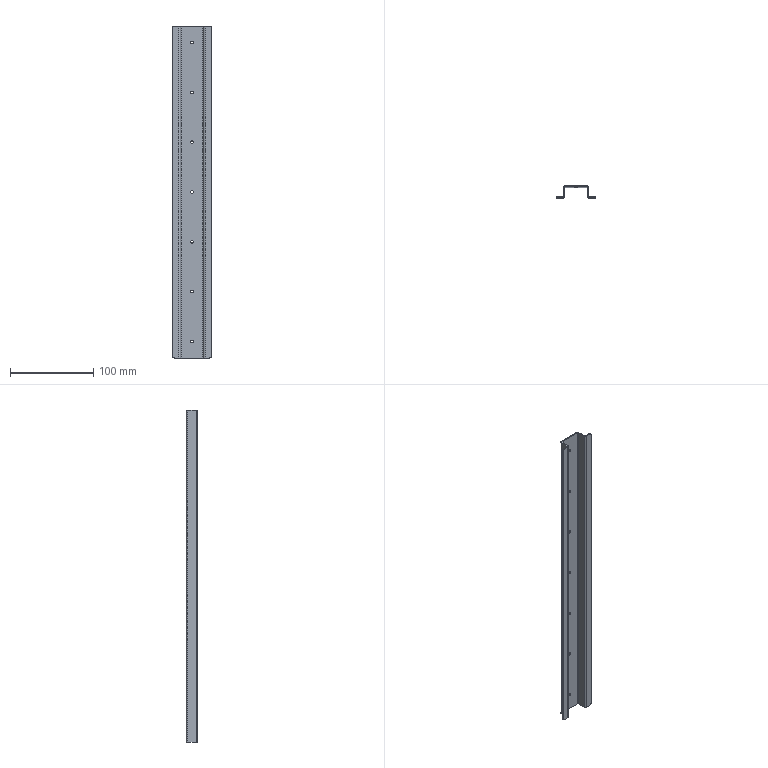Part | SolidWorks | features BaseBody 1 | 1 solid | 56 faces | box 48 x 13.9 x 400 mm | volume 34049 mm3 | plane 30 | cylinder 26 | commonest cylinder face diameters 3.3 x14 1.473 x4 3.873 x4 6 x4
STEP:
#1=CARTESIAN_POINT('',(0.,-1.2,118.35));
#2=VERTEX_POINT('',#1);
#3=CARTESIAN_POINT('',(0.,0.,118.35));
#4=VERTEX_POINT('',#3);
#5=CARTESIAN_POINT('',(0.,0.,118.35));
#6=DIRECTION('',(0.,1.,0.));
#7=VECTOR('',#6,1000.);
#8=LINE('',#5,#7);
#9=EDGE_CURVE('',#2,#4,#8,.T.);
#10=ORIENTED_EDGE('',*,*,#9,.F.);
#11=CARTESIAN_POINT('',(0.,-1.2,121.65));
#12=VERTEX_POINT('',#11);
#13=CARTESIAN_POINT('',(0.,-1.2,120.));
#14=DIRECTION('',(0.,1.,0.));
#15=DIRECTION('',(-1.,0.,0.));
#16=AXIS2_PLACEMENT_3D('',#13,#14,#15);
#17=CIRCLE('',#16,1.65);
#18=EDGE_CURVE('',#12,#2,#17,.T.);
#19=ORIENTED_EDGE('',*,*,#18,.F.);
#20=CARTESIAN_POINT('',(0.,0.,121.65));
#21=VERTEX_POINT('',#20);
#22=CARTESIAN_POINT('',(0.,0.,121.65));
#23=DIRECTION('',(0.,1.,0.));
#24=VECTOR('',#23,1000.);
#25=LINE('',#22,#24);
#26=EDGE_CURVE('',#12,#21,#25,.T.);
#27=ORIENTED_EDGE('',*,*,#26,.T.);
#28=CARTESIAN_POINT('',(0.,0.,120.));
#29=DIRECTION('',(0.,1.,0.));
#30=DIRECTION('',(0.,0.,1.));
#31=AXIS2_PLACEMENT_3D('',#28,#29,#30);
#32=CIRCLE('',#31,1.65);
#33=EDGE_CURVE('',#21,#4,#32,.T.);
#34=ORIENTED_EDGE('',*,*,#33,.T.);
#35=EDGE_LOOP('',(#10,#19,#27,#34));
#36=FACE_OUTER_BOUND('',#35,.T.);
#37=CARTESIAN_POINT('',(0.,0.,120.));
#38=DIRECTION('',(0.,1.,0.));
#39=DIRECTION('',(0.,0.,1.));
#40=AXIS2_PLACEMENT_3D('',#37,#38,#39);
#41=CYLINDRICAL_SURFACE('',#40,1.65);
#42=ADVANCED_FACE('',(#36),#41,.F.);
#43=CARTESIAN_POINT('',(0.,-1.2,58.35));
#44=VERTEX_POINT('',#43);
#45=CARTESIAN_POINT('',(0.,0.,58.35));
#46=VERTEX_POINT('',#45);
#47=CARTESIAN_POINT('',(0.,0.,58.35));
#48=DIRECTION('',(0.,1.,0.));
#49=VECTOR('',#48,1000.);
#50=LINE('',#47,#49);
#51=EDGE_CURVE('',#44,#46,#50,.T.);
#52=ORIENTED_EDGE('',*,*,#51,.F.);
#53=CARTESIAN_POINT('',(0.,-1.2,61.65));
#54=VERTEX_POINT('',#53);
#55=CARTESIAN_POINT('',(0.,-1.2,60.));
#56=DIRECTION('',(0.,1.,0.));
#57=DIRECTION('',(-1.,0.,0.));
#58=AXIS2_PLACEMENT_3D('',#55,#56,#57);
#59=CIRCLE('',#58,1.65);
#60=EDGE_CURVE('',#54,#44,#59,.T.);
#61=ORIENTED_EDGE('',*,*,#60,.F.);
#62=CARTESIAN_POINT('',(0.,0.,61.65));
#63=VERTEX_POINT('',#62);
#64=CARTESIAN_POINT('',(0.,0.,61.65));
#65=DIRECTION('',(0.,1.,0.));
#66=VECTOR('',#65,1000.);
#67=LINE('',#64,#66);
#68=EDGE_CURVE('',#54,#63,#67,.T.);
#69=ORIENTED_EDGE('',*,*,#68,.T.);
#70=CARTESIAN_POINT('',(0.,0.,60.));
#71=DIRECTION('',(0.,1.,0.));
#72=DIRECTION('',(0.,0.,1.));
#73=AXIS2_PLACEMENT_3D('',#70,#71,#72);
#74=CIRCLE('',#73,1.65);
#75=EDGE_CURVE('',#63,#46,#74,.T.);
#76=ORIENTED_EDGE('',*,*,#75,.T.);
#77=EDGE_LOOP('',(#52,#61,#69,#76));
#78=FACE_OUTER_BOUND('',#77,.T.);
#79=CARTESIAN_POINT('',(0.,0.,60.));
#80=DIRECTION('',(0.,1.,0.));
#81=DIRECTION('',(0.,0.,1.));
#82=AXIS2_PLACEMENT_3D('',#79,#80,#81);
#83=CYLINDRICAL_SURFACE('',#82,1.65);
#84=ADVANCED_FACE('',(#78),#83,.F.);
#85=CARTESIAN_POINT('',(0.,-1.2,-1.65));
#86=VERTEX_POINT('',#85);
#87=CARTESIAN_POINT('',(0.,0.,-1.65));
#88=VERTEX_POINT('',#87);
#89=CARTESIAN_POINT('',(0.,0.,-1.65));
#90=DIRECTION('',(0.,1.,0.));
#91=VECTOR('',#90,1000.);
#92=LINE('',#89,#91);
#93=EDGE_CURVE('',#86,#88,#92,.T.);
#94=ORIENTED_EDGE('',*,*,#93,.F.);
#95=CARTESIAN_POINT('',(0.,-1.2,1.65));
#96=VERTEX_POINT('',#95);
#97=CARTESIAN_POINT('',(0.,-1.2,0.));
#98=DIRECTION('',(0.,1.,0.));
#99=DIRECTION('',(-1.,0.,0.));
#100=AXIS2_PLACEMENT_3D('',#97,#98,#99);
#101=CIRCLE('',#100,1.65);
#102=EDGE_CURVE('',#96,#86,#101,.T.);
#103=ORIENTED_EDGE('',*,*,#102,.F.);
#104=CARTESIAN_POINT('',(0.,0.,1.65));
#105=VERTEX_POINT('',#104);
#106=CARTESIAN_POINT('',(0.,0.,1.65));
#107=DIRECTION('',(0.,1.,0.));
#108=VECTOR('',#107,1000.);
#109=LINE('',#106,#108);
#110=EDGE_CURVE('',#96,#105,#109,.T.);
#111=ORIENTED_EDGE('',*,*,#110,.T.);
#112=CARTESIAN_POINT('',(0.,0.,0.));
#113=DIRECTION('',(0.,1.,0.));
#114=DIRECTION('',(0.,0.,1.));
#115=AXIS2_PLACEMENT_3D('',#112,#113,#114);
#116=CIRCLE('',#115,1.65);
#117=EDGE_CURVE('',#105,#88,#116,.T.);
#118=ORIENTED_EDGE('',*,*,#117,.T.);
#119=EDGE_LOOP('',(#94,#103,#111,#118));
#120=FACE_OUTER_BOUND('',#119,.T.);
#121=CARTESIAN_POINT('',(0.,0.,0.));
#122=DIRECTION('',(0.,1.,0.));
#123=DIRECTION('',(0.,0.,1.));
#124=AXIS2_PLACEMENT_3D('',#121,#122,#123);
#125=CYLINDRICAL_SURFACE('',#124,1.65);
#126=ADVANCED_FACE('',(#120),#125,.F.);
#127=CARTESIAN_POINT('',(0.,-1.2,-61.65));
#128=VERTEX_POINT('',#127);
#129=CARTESIAN_POINT('',(0.,0.,-61.65));
#130=VERTEX_POINT('',#129);
#131=CARTESIAN_POINT('',(0.,0.,-61.65));
#132=DIRECTION('',(0.,1.,0.));
#133=VECTOR('',#132,1000.);
#134=LINE('',#131,#133);
#135=EDGE_CURVE('',#128,#130,#134,.T.);
#136=ORIENTED_EDGE('',*,*,#135,.F.);
#137=CARTESIAN_POINT('',(0.,-1.2,-58.35));
#138=VERTEX_POINT('',#137);
#139=CARTESIAN_POINT('',(0.,-1.2,-60.));
#140=DIRECTION('',(0.,1.,0.));
#141=DIRECTION('',(-1.,0.,0.));
#142=AXIS2_PLACEMENT_3D('',#139,#140,#141);
#143=CIRCLE('',#142,1.65);
#144=EDGE_CURVE('',#138,#128,#143,.T.);
#145=ORIENTED_EDGE('',*,*,#144,.F.);
#146=CARTESIAN_POINT('',(0.,0.,-58.35));
#147=VERTEX_POINT('',#146);
#148=CARTESIAN_POINT('',(0.,0.,-58.35));
#149=DIRECTION('',(0.,1.,0.));
#150=VECTOR('',#149,1000.);
#151=LINE('',#148,#150);
#152=EDGE_CURVE('',#138,#147,#151,.T.);
#153=ORIENTED_EDGE('',*,*,#152,.T.);
#154=CARTESIAN_POINT('',(0.,0.,-60.));
#155=DIRECTION('',(0.,1.,0.));
#156=DIRECTION('',(0.,0.,1.));
#157=AXIS2_PLACEMENT_3D('',#154,#155,#156);
#158=CIRCLE('',#157,1.65);
#159=EDGE_CURVE('',#147,#130,#158,.T.);
#160=ORIENTED_EDGE('',*,*,#159,.T.);
#161=EDGE_LOOP('',(#136,#145,#153,#160));
#162=FACE_OUTER_BOUND('',#161,.T.);
#163=CARTESIAN_POINT('',(0.,0.,-60.));
#164=DIRECTION('',(0.,1.,0.));
#165=DIRECTION('',(0.,0.,1.));
#166=AXIS2_PLACEMENT_3D('',#163,#164,#165);
#167=CYLINDRICAL_SURFACE('',#166,1.65);
#168=ADVANCED_FACE('',(#162),#167,.F.);
#169=CARTESIAN_POINT('',(0.,-1.2,-121.65));
#170=VERTEX_POINT('',#169);
#171=CARTESIAN_POINT('',(0.,0.,-121.65));
#172=VERTEX_POINT('',#171);
#173=CARTESIAN_POINT('',(0.,0.,-121.65));
#174=DIRECTION('',(0.,1.,0.));
#175=VECTOR('',#174,1000.);
#176=LINE('',#173,#175);
#177=EDGE_CURVE('',#170,#172,#176,.T.);
#178=ORIENTED_EDGE('',*,*,#177,.F.);
#179=CARTESIAN_POINT('',(0.,-1.2,-118.35));
#180=VERTEX_POINT('',#179);
#181=CARTESIAN_POINT('',(0.,-1.2,-120.));
#182=DIRECTION('',(0.,1.,0.));
#183=DIRECTION('',(-1.,0.,0.));
#184=AXIS2_PLACEMENT_3D('',#181,#182,#183);
#185=CIRCLE('',#184,1.65);
#186=EDGE_CURVE('',#180,#170,#185,.T.);
#187=ORIENTED_EDGE('',*,*,#186,.F.);
#188=CARTESIAN_POINT('',(0.,0.,-118.35));
#189=VERTEX_POINT('',#188);
#190=CARTESIAN_POINT('',(0.,0.,-118.35));
#191=DIRECTION('',(0.,1.,0.));
#192=VECTOR('',#191,1000.);
#193=LINE('',#190,#192);
#194=EDGE_CURVE('',#180,#189,#193,.T.);
#195=ORIENTED_EDGE('',*,*,#194,.T.);
#196=CARTESIAN_POINT('',(0.,0.,-120.));
#197=DIRECTION('',(0.,1.,0.));
#198=DIRECTION('',(0.,0.,1.));
#199=AXIS2_PLACEMENT_3D('',#196,#197,#198);
#200=CIRCLE('',#199,1.65);
#201=EDGE_CURVE('',#189,#172,#200,.T.);
#202=ORIENTED_EDGE('',*,*,#201,.T.);
#203=EDGE_LOOP('',(#178,#187,#195,#202));
#204=FACE_OUTER_BOUND('',#203,.T.);
#205=CARTESIAN_POINT('',(0.,0.,-120.));
#206=DIRECTION('',(0.,1.,0.));
#207=DIRECTION('',(0.,0.,1.));
#208=AXIS2_PLACEMENT_3D('',#205,#206,#207);
#209=CYLINDRICAL_SURFACE('',#208,1.65);
#210=ADVANCED_FACE('',(#204),#209,.F.);
#211=CARTESIAN_POINT('',(0.,-1.2,-181.65));
#212=VERTEX_POINT('',#211);
#213=CARTESIAN_POINT('',(0.,0.,-181.65));
#214=VERTEX_POINT('',#213);
#215=CARTESIAN_POINT('',(0.,0.,-181.65));
#216=DIRECTION('',(0.,1.,0.));
#217=VECTOR('',#216,1000.);
#218=LINE('',#215,#217);
#219=EDGE_CURVE('',#212,#214,#218,.T.);
#220=ORIENTED_EDGE('',*,*,#219,.F.);
#221=CARTESIAN_POINT('',(0.,-1.2,-178.35));
#222=VERTEX_POINT('',#221);
#223=CARTESIAN_POINT('',(0.,-1.2,-180.));
#224=DIRECTION('',(0.,1.,0.));
#225=DIRECTION('',(-1.,0.,0.));
#226=AXIS2_PLACEMENT_3D('',#223,#224,#225);
#227=CIRCLE('',#226,1.65);
#228=EDGE_CURVE('',#222,#212,#227,.T.);
#229=ORIENTED_EDGE('',*,*,#228,.F.);
#230=CARTESIAN_POINT('',(0.,0.,-178.35));
#231=VERTEX_POINT('',#230);
#232=CARTESIAN_POINT('',(0.,0.,-178.35));
#233=DIRECTION('',(0.,1.,0.));
#234=VECTOR('',#233,1000.);
#235=LINE('',#232,#234);
#236=EDGE_CURVE('',#222,#231,#235,.T.);
#237=ORIENTED_EDGE('',*,*,#236,.T.);
#238=CARTESIAN_POINT('',(0.,0.,-180.));
#239=DIRECTION('',(0.,1.,0.));
#240=DIRECTION('',(0.,0.,1.));
#241=AXIS2_PLACEMENT_3D('',#238,#239,#240);
#242=CIRCLE('',#241,1.65);
#243=EDGE_CURVE('',#231,#214,#242,.T.);
#244=ORIENTED_EDGE('',*,*,#243,.T.);
#245=EDGE_LOOP('',(#220,#229,#237,#244));
#246=FACE_OUTER_BOUND('',#245,.T.);
#247=CARTESIAN_POINT('',(0.,0.,-180.));
#248=DIRECTION('',(0.,1.,0.));
#249=DIRECTION('',(0.,0.,1.));
#250=AXIS2_PLACEMENT_3D('',#247,#248,#249);
#251=CYLINDRICAL_SURFACE('',#250,1.65);
#252=ADVANCED_FACE('',(#246),#251,.F.);
#253=CARTESIAN_POINT('',(0.,-1.2,178.35));
#254=VERTEX_POINT('',#253);
#255=CARTESIAN_POINT('',(0.,0.,178.35));
#256=VERTEX_POINT('',#255);
#257=CARTESIAN_POINT('',(0.,0.,178.35));
#258=DIRECTION('',(0.,1.,0.));
#259=VECTOR('',#258,1000.);
#260=LINE('',#257,#259);
#261=EDGE_CURVE('',#254,#256,#260,.T.);
#262=ORIENTED_EDGE('',*,*,#261,.F.);
#263=CARTESIAN_POINT('',(0.,-1.2,181.65));
#264=VERTEX_POINT('',#263);
#265=CARTESIAN_POINT('',(0.,-1.2,180.));
#266=DIRECTION('',(0.,1.,0.));
#267=DIRECTION('',(-1.,0.,0.));
#268=AXIS2_PLACEMENT_3D('',#265,#266,#267);
#269=CIRCLE('',#268,1.65);
#270=EDGE_CURVE('',#264,#254,#269,.T.);
#271=ORIENTED_EDGE('',*,*,#270,.F.);
#272=CARTESIAN_POINT('',(0.,0.,181.65));
#273=VERTEX_POINT('',#272);
#274=CARTESIAN_POINT('',(0.,0.,181.65));
#275=DIRECTION('',(0.,1.,0.));
#276=VECTOR('',#275,1000.);
#277=LINE('',#274,#276);
#278=EDGE_CURVE('',#264,#273,#277,.T.);
#279=ORIENTED_EDGE('',*,*,#278,.T.);
#280=CARTESIAN_POINT('',(0.,0.,180.));
#281=DIRECTION('',(0.,1.,0.));
#282=DIRECTION('',(0.,0.,1.));
#283=AXIS2_PLACEMENT_3D('',#280,#281,#282);
#284=CIRCLE('',#283,1.65);
#285=EDGE_CURVE('',#273,#256,#284,.T.);
#286=ORIENTED_EDGE('',*,*,#285,.T.);
#287=EDGE_LOOP('',(#262,#271,#279,#286));
#288=FACE_OUTER_BOUND('',#287,.T.);
#289=CARTESIAN_POINT('',(0.,0.,180.));
#290=DIRECTION('',(0.,1.,0.));
#291=DIRECTION('',(0.,0.,1.));
#292=AXIS2_PLACEMENT_3D('',#289,#290,#291);
#293=CYLINDRICAL_SURFACE('',#292,1.65);
#294=ADVANCED_FACE('',(#288),#293,.F.);
#295=CARTESIAN_POINT('',(-24.,-13.9,-197.));
#296=VERTEX_POINT('',#295);
#297=CARTESIAN_POINT('',(-21.,-13.9,-200.));
#298=VERTEX_POINT('',#297);
#299=CARTESIAN_POINT('',(-21.,-13.9,-197.));
#300=DIRECTION('',(0.,-1.,0.));
#301=DIRECTION('',(-1.,0.,0.));
#302=AXIS2_PLACEMENT_3D('',#299,#300,#301);
#303=CIRCLE('',#302,3.);
#304=EDGE_CURVE('',#296,#298,#303,.T.);
#305=ORIENTED_EDGE('',*,*,#304,.F.);
#306=CARTESIAN_POINT('',(-24.,-12.7,-197.));
#307=VERTEX_POINT('',#306);
#308=CARTESIAN_POINT('',(-24.,-13.9,-197.));
#309=DIRECTION('',(0.,-1.,0.));
#310=VECTOR('',#309,1000.);
#311=LINE('',#308,#310);
#312=EDGE_CURVE('',#307,#296,#311,.T.);
#313=ORIENTED_EDGE('',*,*,#312,.F.);
#314=CARTESIAN_POINT('',(-21.,-12.7,-200.));
#315=VERTEX_POINT('',#314);
#316=CARTESIAN_POINT('',(-21.,-12.7,-197.));
#317=DIRECTION('',(0.,1.,0.));
#318=DIRECTION('',(-1.,0.,0.));
#319=AXIS2_PLACEMENT_3D('',#316,#317,#318);
#320=CIRCLE('',#319,3.);
#321=EDGE_CURVE('',#315,#307,#320,.T.);
#322=ORIENTED_EDGE('',*,*,#321,.F.);
#323=CARTESIAN_POINT('',(-21.,-11.963,-200.));
#324=DIRECTION('',(0.,1.,0.));
#325=VECTOR('',#324,1000.);
#326=LINE('',#323,#325);
#327=EDGE_CURVE('',#298,#315,#326,.T.);
#328=ORIENTED_EDGE('',*,*,#327,.F.);
#329=EDGE_LOOP('',(#305,#313,#322,#328));
#330=FACE_OUTER_BOUND('',#329,.T.);
#331=CARTESIAN_POINT('',(-21.,-11.963,-197.));
#332=DIRECTION('',(0.,1.,0.));
#333=DIRECTION('',(0.,0.,1.));
#334=AXIS2_PLACEMENT_3D('',#331,#332,#333);
#335=CYLINDRICAL_SURFACE('',#334,3.);
#336=ADVANCED_FACE('',(#330),#335,.T.);
#337=CARTESIAN_POINT('',(24.,-12.7,-197.));
#338=VERTEX_POINT('',#337);
#339=CARTESIAN_POINT('',(21.,-12.7,-200.));
#340=VERTEX_POINT('',#339);
#341=CARTESIAN_POINT('',(21.,-12.7,-197.));
#342=DIRECTION('',(0.,1.,0.));
#343=DIRECTION('',(-1.,0.,0.));
#344=AXIS2_PLACEMENT_3D('',#341,#342,#343);
#345=CIRCLE('',#344,3.);
#346=EDGE_CURVE('',#338,#340,#345,.T.);
#347=ORIENTED_EDGE('',*,*,#346,.F.);
#348=CARTESIAN_POINT('',(24.,-13.9,-197.));
#349=VERTEX_POINT('',#348);
#350=CARTESIAN_POINT('',(24.,-12.7,-197.));
#351=DIRECTION('',(0.,1.,0.));
#352=VECTOR('',#351,1000.);
#353=LINE('',#350,#352);
#354=EDGE_CURVE('',#349,#338,#353,.T.);
#355=ORIENTED_EDGE('',*,*,#354,.F.);
#356=CARTESIAN_POINT('',(21.,-13.9,-200.));
#357=VERTEX_POINT('',#356);
#358=CARTESIAN_POINT('',(21.,-13.9,-197.));
#359=DIRECTION('',(0.,-1.,0.));
#360=DIRECTION('',(-1.,0.,0.));
#361=AXIS2_PLACEMENT_3D('',#358,#359,#360);
#362=CIRCLE('',#361,3.);
#363=EDGE_CURVE('',#357,#349,#362,.T.);
#364=ORIENTED_EDGE('',*,*,#363,.F.);
#365=CARTESIAN_POINT('',(21.,-11.963,-200.));
#366=DIRECTION('',(0.,-1.,0.));
#367=VECTOR('',#366,1000.);
#368=LINE('',#365,#367);
#369=EDGE_CURVE('',#340,#357,#368,.T.);
#370=ORIENTED_EDGE('',*,*,#369,.F.);
#371=EDGE_LOOP('',(#347,#355,#364,#370));
#372=FACE_OUTER_BOUND('',#371,.T.);
#373=CARTESIAN_POINT('',(21.,-11.963,-197.));
#374=DIRECTION('',(0.,-1.,0.));
#375=DIRECTION('',(0.,0.,-1.));
#376=AXIS2_PLACEMENT_3D('',#373,#374,#375);
#377=CYLINDRICAL_SURFACE('',#376,3.);
#378=ADVANCED_FACE('',(#372),#377,.T.);
#379=CARTESIAN_POINT('',(-21.,-13.9,200.));
#380=VERTEX_POINT('',#379);
#381=CARTESIAN_POINT('',(-24.,-13.9,197.));
#382=VERTEX_POINT('',#381);
#383=CARTESIAN_POINT('',(-21.,-13.9,197.));
#384=DIRECTION('',(0.,-1.,0.));
#385=DIRECTION('',(-1.,0.,0.));
#386=AXIS2_PLACEMENT_3D('',#383,#384,#385);
#387=CIRCLE('',#386,3.);
#388=EDGE_CURVE('',#380,#382,#387,.T.);
#389=ORIENTED_EDGE('',*,*,#388,.F.);
#390=CARTESIAN_POINT('',(-21.,-12.7,200.));
#391=VERTEX_POINT('',#390);
#392=CARTESIAN_POINT('',(-21.,-13.9,200.));
#393=DIRECTION('',(0.,-1.,0.));
#394=VECTOR('',#393,1000.);
#395=LINE('',#392,#394);
#396=EDGE_CURVE('',#391,#380,#395,.T.);
#397=ORIENTED_EDGE('',*,*,#396,.F.);
#398=CARTESIAN_POINT('',(-24.,-12.7,197.));
#399=VERTEX_POINT('',#398);
#400=CARTESIAN_POINT('',(-21.,-12.7,197.));
#401=DIRECTION('',(0.,1.,0.));
#402=DIRECTION('',(-1.,0.,0.));
#403=AXIS2_PLACEMENT_3D('',#400,#401,#402);
#404=CIRCLE('',#403,3.);
#405=EDGE_CURVE('',#399,#391,#404,.T.);
#406=ORIENTED_EDGE('',*,*,#405,.F.);
#407=CARTESIAN_POINT('',(-24.,-12.7,197.));
#408=DIRECTION('',(0.,1.,0.));
#409=VECTOR('',#408,1000.);
#410=LINE('',#407,#409);
#411=EDGE_CURVE('',#382,#399,#410,.T.);
#412=ORIENTED_EDGE('',*,*,#411,.F.);
#413=EDGE_LOOP('',(#389,#397,#406,#412));
#414=FACE_OUTER_BOUND('',#413,.T.);
#415=CARTESIAN_POINT('',(-21.,-13.9,197.));
#416=DIRECTION('',(0.,-1.,0.));
#417=DIRECTION('',(0.,0.,-1.));
#418=AXIS2_PLACEMENT_3D('',#415,#416,#417);
#419=CYLINDRICAL_SURFACE('',#418,3.);
#420=ADVANCED_FACE('',(#414),#419,.T.);
#421=CARTESIAN_POINT('',(21.,-12.7,200.));
#422=VERTEX_POINT('',#421);
#423=CARTESIAN_POINT('',(24.,-12.7,197.));
#424=VERTEX_POINT('',#423);
#425=CARTESIAN_POINT('',(21.,-12.7,197.));
#426=DIRECTION('',(0.,1.,0.));
#427=DIRECTION('',(-1.,0.,0.));
#428=AXIS2_PLACEMENT_3D('',#425,#426,#427);
#429=CIRCLE('',#428,3.);
#430=EDGE_CURVE('',#422,#424,#429,.T.);
#431=ORIENTED_EDGE('',*,*,#430,.F.);
#432=CARTESIAN_POINT('',(21.,-13.9,200.));
#433=VERTEX_POINT('',#432);
#434=CARTESIAN_POINT('',(21.,-11.963,200.));
#435=DIRECTION('',(0.,1.,0.));
#436=VECTOR('',#435,1000.);
#437=LINE('',#434,#436);
#438=EDGE_CURVE('',#433,#422,#437,.T.);
#439=ORIENTED_EDGE('',*,*,#438,.F.);
#440=CARTESIAN_POINT('',(24.,-13.9,197.));
#441=VERTEX_POINT('',#440);
#442=CARTESIAN_POINT('',(21.,-13.9,197.));
#443=DIRECTION('',(0.,-1.,0.));
#444=DIRECTION('',(-1.,0.,0.));
#445=AXIS2_PLACEMENT_3D('',#442,#443,#444);
#446=CIRCLE('',#445,3.);
#447=EDGE_CURVE('',#441,#433,#446,.T.);
#448=ORIENTED_EDGE('',*,*,#447,.F.);
#449=CARTESIAN_POINT('',(24.,-12.7,197.));
#450=DIRECTION('',(0.,-1.,0.));
#451=VECTOR('',#450,1000.);
#452=LINE('',#449,#451);
#453=EDGE_CURVE('',#424,#441,#452,.T.);
#454=ORIENTED_EDGE('',*,*,#453,.F.);
#455=EDGE_LOOP('',(#431,#439,#448,#454));
#456=FACE_OUTER_BOUND('',#455,.T.);
#457=CARTESIAN_POINT('',(21.,-12.7,197.));
#458=DIRECTION('',(0.,-1.,0.));
#459=DIRECTION('',(0.,0.,-1.));
#460=AXIS2_PLACEMENT_3D('',#457,#458,#459);
#461=CYLINDRICAL_SURFACE('',#460,3.);
#462=ADVANCED_FACE('',(#456),#461,.T.);
#463=CARTESIAN_POINT('',(15.737,-12.7,-200.));
#464=VERTEX_POINT('',#463);
#465=CARTESIAN_POINT('',(15.,-12.7,-200.));
#466=DIRECTION('',(1.,0.,0.));
#467=VECTOR('',#466,1000.);
#468=LINE('',#465,#467);
#469=EDGE_CURVE('',#464,#340,#468,.T.);
#470=ORIENTED_EDGE('',*,*,#469,.T.);
#471=ORIENTED_EDGE('',*,*,#369,.T.);
#472=CARTESIAN_POINT('',(15.737,-13.9,-200.));
#473=VERTEX_POINT('',#472);
#474=CARTESIAN_POINT('',(15.,-13.9,-200.));
#475=DIRECTION('',(1.,0.,0.));
#476=VECTOR('',#475,1000.);
#477=LINE('',#474,#476);
#478=EDGE_CURVE('',#473,#357,#477,.T.);
#479=ORIENTED_EDGE('',*,*,#478,.F.);
#480=CARTESIAN_POINT('',(15.737,-13.9,-200.));
#481=DIRECTION('',(0.,1.,0.));
#482=VECTOR('',#481,1000.);
#483=LINE('',#480,#482);
#484=EDGE_CURVE('',#473,#464,#483,.T.);
#485=ORIENTED_EDGE('',*,*,#484,.T.);
#486=EDGE_LOOP('',(#470,#471,#479,#485));
#487=FACE_OUTER_BOUND('',#486,.T.);
#488=CARTESIAN_POINT('',(15.737,-11.963,-200.));
#489=DIRECTION('',(0.,0.,-1.));
#490=DIRECTION('',(0.,-1.,0.));
#491=AXIS2_PLACEMENT_3D('',#488,#489,#490);
#492=PLANE('',#491);
#493=ADVANCED_FACE('',(#487),#492,.T.);
#494=CARTESIAN_POINT('',(-15.737,-12.7,200.));
#495=VERTEX_POINT('',#494);
#496=CARTESIAN_POINT('',(-15.,-12.7,200.));
#497=DIRECTION('',(1.,0.,0.));
#498=VECTOR('',#497,1000.);
#499=LINE('',#496,#498);
#500=EDGE_CURVE('',#391,#495,#499,.T.);
#501=ORIENTED_EDGE('',*,*,#500,.F.);
#502=ORIENTED_EDGE('',*,*,#396,.T.);
#503=CARTESIAN_POINT('',(-15.737,-13.9,200.));
#504=VERTEX_POINT('',#503);
#505=CARTESIAN_POINT('',(-15.,-13.9,200.));
#506=DIRECTION('',(1.,0.,0.));
#507=VECTOR('',#506,1000.);
#508=LINE('',#505,#507);
#509=EDGE_CURVE('',#380,#504,#508,.T.);
#510=ORIENTED_EDGE('',*,*,#509,.T.);
#511=CARTESIAN_POINT('',(-15.737,-13.9,200.));
#512=DIRECTION('',(0.,1.,0.));
#513=VECTOR('',#512,1000.);
#514=LINE('',#511,#513);
#515=EDGE_CURVE('',#504,#495,#514,.T.);
#516=ORIENTED_EDGE('',*,*,#515,.T.);
#517=EDGE_LOOP('',(#501,#502,#510,#516));
#518=FACE_OUTER_BOUND('',#517,.T.);
#519=CARTESIAN_POINT('',(15.737,-11.963,200.));
#520=DIRECTION('',(0.,0.,-1.));
#521=DIRECTION('',(0.,-1.,0.));
#522=AXIS2_PLACEMENT_3D('',#519,#520,#521);
#523=PLANE('',#522);
#524=ADVANCED_FACE('',(#518),#523,.F.);
#525=CARTESIAN_POINT('',(13.8,-11.963,-200.));
#526=VERTEX_POINT('',#525);
#527=CARTESIAN_POINT('',(15.737,-11.963,-200.));
#528=DIRECTION('',(0.,0.,1.));
#529=DIRECTION('',(1.,0.,0.));
#530=AXIS2_PLACEMENT_3D('',#527,#528,#529);
#531=CIRCLE('',#530,1.937);
#532=EDGE_CURVE('',#526,#473,#531,.T.);
#533=ORIENTED_EDGE('',*,*,#532,.T.);
#534=CARTESIAN_POINT('',(15.737,-13.9,200.));
#535=VERTEX_POINT('',#534);
#536=CARTESIAN_POINT('',(15.737,-13.9,200.));
#537=DIRECTION('',(0.,0.,-1.));
#538=VECTOR('',#537,1000.);
#539=LINE('',#536,#538);
#540=EDGE_CURVE('',#535,#473,#539,.T.);
#541=ORIENTED_EDGE('',*,*,#540,.F.);
#542=CARTESIAN_POINT('',(13.8,-11.963,200.));
#543=VERTEX_POINT('',#542);
#544=CARTESIAN_POINT('',(15.737,-11.963,200.));
#545=DIRECTION('',(0.,0.,1.));
#546=DIRECTION('',(1.,0.,0.));
#547=AXIS2_PLACEMENT_3D('',#544,#545,#546);
#548=CIRCLE('',#547,1.937);
#549=EDGE_CURVE('',#543,#535,#548,.T.);
#550=ORIENTED_EDGE('',*,*,#549,.F.);
#551=CARTESIAN_POINT('',(13.8,-11.963,200.));
#552=DIRECTION('',(0.,0.,-1.));
#553=VECTOR('',#552,1000.);
#554=LINE('',#551,#553);
#555=EDGE_CURVE('',#543,#526,#554,.T.);
#556=ORIENTED_EDGE('',*,*,#555,.T.);
#557=EDGE_LOOP('',(#533,#541,#550,#556));
#558=FACE_OUTER_BOUND('',#557,.T.);
#559=CARTESIAN_POINT('',(15.737,-11.963,200.));
#560=DIRECTION('',(0.,0.,-1.));
#561=DIRECTION('',(-1.,0.,0.));
#562=AXIS2_PLACEMENT_3D('',#559,#560,#561);
#563=CYLINDRICAL_SURFACE('',#562,1.937);
#564=ADVANCED_FACE('',(#558),#563,.T.);
#565=CARTESIAN_POINT('',(13.8,-1.937,-200.));
#566=VERTEX_POINT('',#565);
#567=CARTESIAN_POINT('',(13.8,0.,-200.));
#568=DIRECTION('',(0.,-1.,0.));
#569=VECTOR('',#568,1000.);
#570=LINE('',#567,#569);
#571=EDGE_CURVE('',#566,#526,#570,.T.);
#572=ORIENTED_EDGE('',*,*,#571,.T.);
#573=ORIENTED_EDGE('',*,*,#555,.F.);
#574=CARTESIAN_POINT('',(13.8,-1.937,200.));
#575=VERTEX_POINT('',#574);
#576=CARTESIAN_POINT('',(13.8,0.,200.));
#577=DIRECTION('',(0.,-1.,0.));
#578=VECTOR('',#577,1000.);
#579=LINE('',#576,#578);
#580=EDGE_CURVE('',#575,#543,#579,.T.);
#581=ORIENTED_EDGE('',*,*,#580,.F.);
#582=CARTESIAN_POINT('',(13.8,-1.937,200.));
#583=DIRECTION('',(0.,0.,-1.));
#584=VECTOR('',#583,1000.);
#585=LINE('',#582,#584);
#586=EDGE_CURVE('',#575,#566,#585,.T.);
#587=ORIENTED_EDGE('',*,*,#586,.T.);
#588=EDGE_LOOP('',(#572,#573,#581,#587));
#589=FACE_OUTER_BOUND('',#588,.T.);
#590=CARTESIAN_POINT('',(13.8,0.,200.));
#591=DIRECTION('',(1.,0.,0.));
#592=DIRECTION('',(0.,1.,0.));
#593=AXIS2_PLACEMENT_3D('',#590,#591,#592);
#594=PLANE('',#593);
#595=ADVANCED_FACE('',(#589),#594,.F.);
#596=CARTESIAN_POINT('',(13.063,-1.2,-200.));
#597=VERTEX_POINT('',#596);
#598=CARTESIAN_POINT('',(13.063,-1.937,-200.));
#599=DIRECTION('',(0.,0.,-1.));
#600=DIRECTION('',(1.,0.,0.));
#601=AXIS2_PLACEMENT_3D('',#598,#599,#600);
#602=CIRCLE('',#601,0.7366);
#603=EDGE_CURVE('',#597,#566,#602,.T.);
#604=ORIENTED_EDGE('',*,*,#603,.T.);
#605=ORIENTED_EDGE('',*,*,#586,.F.);
#606=CARTESIAN_POINT('',(13.063,-1.2,200.));
#607=VERTEX_POINT('',#606);
#608=CARTESIAN_POINT('',(13.063,-1.937,200.));
#609=DIRECTION('',(0.,0.,-1.));
#610=DIRECTION('',(1.,0.,0.));
#611=AXIS2_PLACEMENT_3D('',#608,#609,#610);
#612=CIRCLE('',#611,0.7366);
#613=EDGE_CURVE('',#607,#575,#612,.T.);
#614=ORIENTED_EDGE('',*,*,#613,.F.);
#615=CARTESIAN_POINT('',(13.063,-1.2,200.));
#616=DIRECTION('',(0.,0.,-1.));
#617=VECTOR('',#616,1000.);
#618=LINE('',#615,#617);
#619=EDGE_CURVE('',#607,#597,#618,.T.);
#620=ORIENTED_EDGE('',*,*,#619,.T.);
#621=EDGE_LOOP('',(#604,#605,#614,#620));
#622=FACE_OUTER_BOUND('',#621,.T.);
#623=CARTESIAN_POINT('',(13.063,-1.937,200.));
#624=DIRECTION('',(0.,0.,-1.));
#625=DIRECTION('',(-1.,0.,0.));
#626=AXIS2_PLACEMENT_3D('',#623,#624,#625);
#627=CYLINDRICAL_SURFACE('',#626,0.7366);
#628=ADVANCED_FACE('',(#622),#627,.F.);
#629=ORIENTED_EDGE('',*,*,#270,.T.);
#630=CARTESIAN_POINT('',(0.,-1.2,180.));
#631=DIRECTION('',(0.,1.,0.));
#632=DIRECTION('',(-1.,0.,0.));
#633=AXIS2_PLACEMENT_3D('',#630,#631,#632);
#634=CIRCLE('',#633,1.65);
#635=EDGE_CURVE('',#254,#264,#634,.T.);
#636=ORIENTED_EDGE('',*,*,#635,.T.);
#637=EDGE_LOOP('',(#629,#636));
#638=FACE_BOUND('',#637,.T.);
#639=ORIENTED_EDGE('',*,*,#228,.T.);
#640=CARTESIAN_POINT('',(0.,-1.2,-180.));
#641=DIRECTION('',(0.,1.,0.));
#642=DIRECTION('',(-1.,0.,0.));
#643=AXIS2_PLACEMENT_3D('',#640,#641,#642);
#644=CIRCLE('',#643,1.65);
#645=EDGE_CURVE('',#212,#222,#644,.T.);
#646=ORIENTED_EDGE('',*,*,#645,.T.);
#647=EDGE_LOOP('',(#639,#646));
#648=FACE_BOUND('',#647,.T.);
#649=ORIENTED_EDGE('',*,*,#186,.T.);
#650=CARTESIAN_POINT('',(0.,-1.2,-120.));
#651=DIRECTION('',(0.,1.,0.));
#652=DIRECTION('',(-1.,0.,0.));
#653=AXIS2_PLACEMENT_3D('',#650,#651,#652);
#654=CIRCLE('',#653,1.65);
#655=EDGE_CURVE('',#170,#180,#654,.T.);
#656=ORIENTED_EDGE('',*,*,#655,.T.);
#657=EDGE_LOOP('',(#649,#656));
#658=FACE_BOUND('',#657,.T.);
#659=ORIENTED_EDGE('',*,*,#144,.T.);
#660=CARTESIAN_POINT('',(0.,-1.2,-60.));
#661=DIRECTION('',(0.,1.,0.));
#662=DIRECTION('',(-1.,0.,0.));
#663=AXIS2_PLACEMENT_3D('',#660,#661,#662);
#664=CIRCLE('',#663,1.65);
#665=EDGE_CURVE('',#128,#138,#664,.T.);
#666=ORIENTED_EDGE('',*,*,#665,.T.);
#667=EDGE_LOOP('',(#659,#666));
#668=FACE_BOUND('',#667,.T.);
#669=ORIENTED_EDGE('',*,*,#102,.T.);
#670=CARTESIAN_POINT('',(0.,-1.2,0.));
#671=DIRECTION('',(0.,1.,0.));
#672=DIRECTION('',(-1.,0.,0.));
#673=AXIS2_PLACEMENT_3D('',#670,#671,#672);
#674=CIRCLE('',#673,1.65);
#675=EDGE_CURVE('',#86,#96,#674,.T.);
#676=ORIENTED_EDGE('',*,*,#675,.T.);
#677=EDGE_LOOP('',(#669,#676));
#678=FACE_BOUND('',#677,.T.);
#679=ORIENTED_EDGE('',*,*,#60,.T.);
#680=CARTESIAN_POINT('',(0.,-1.2,60.));
#681=DIRECTION('',(0.,1.,0.));
#682=DIRECTION('',(-1.,0.,0.));
#683=AXIS2_PLACEMENT_3D('',#680,#681,#682);
#684=CIRCLE('',#683,1.65);
#685=EDGE_CURVE('',#44,#54,#684,.T.);
#686=ORIENTED_EDGE('',*,*,#685,.T.);
#687=EDGE_LOOP('',(#679,#686));
#688=FACE_BOUND('',#687,.T.);
#689=ORIENTED_EDGE('',*,*,#18,.T.);
#690=CARTESIAN_POINT('',(0.,-1.2,120.));
#691=DIRECTION('',(0.,1.,0.));
#692=DIRECTION('',(-1.,0.,0.));
#693=AXIS2_PLACEMENT_3D('',#690,#691,#692);
#694=CIRCLE('',#693,1.65);
#695=EDGE_CURVE('',#2,#12,#694,.T.);
#696=ORIENTED_EDGE('',*,*,#695,.T.);
#697=EDGE_LOOP('',(#689,#696));
#698=FACE_BOUND('',#697,.T.);
#699=CARTESIAN_POINT('',(-13.063,-1.2,-200.));
#700=VERTEX_POINT('',#699);
#701=CARTESIAN_POINT('',(-15.,-1.2,-200.));
#702=DIRECTION('',(1.,0.,0.));
#703=VECTOR('',#702,1000.);
#704=LINE('',#701,#703);
#705=EDGE_CURVE('',#700,#597,#704,.T.);
#706=ORIENTED_EDGE('',*,*,#705,.T.);
#707=ORIENTED_EDGE('',*,*,#619,.F.);
#708=CARTESIAN_POINT('',(-13.063,-1.2,200.));
#709=VERTEX_POINT('',#708);
#710=CARTESIAN_POINT('',(-15.,-1.2,200.));
#711=DIRECTION('',(1.,0.,0.));
#712=VECTOR('',#711,1000.);
#713=LINE('',#710,#712);
#714=EDGE_CURVE('',#709,#607,#713,.T.);
#715=ORIENTED_EDGE('',*,*,#714,.F.);
#716=CARTESIAN_POINT('',(-13.063,-1.2,200.));
#717=DIRECTION('',(0.,0.,-1.));
#718=VECTOR('',#717,1000.);
#719=LINE('',#716,#718);
#720=EDGE_CURVE('',#709,#700,#719,.T.);
#721=ORIENTED_EDGE('',*,*,#720,.T.);
#722=EDGE_LOOP('',(#706,#707,#715,#721));
#723=FACE_OUTER_BOUND('',#722,.T.);
#724=CARTESIAN_POINT('',(-15.,-1.2,200.));
#725=DIRECTION('',(0.,1.,0.));
#726=DIRECTION('',(1.,0.,0.));
#727=AXIS2_PLACEMENT_3D('',#724,#725,#726);
#728=PLANE('',#727);
#729=ADVANCED_FACE('',(#638,#648,#658,#668,#678,#688,#698,#723),#728,.F.);
#730=CARTESIAN_POINT('',(-13.8,-1.937,-200.));
#731=VERTEX_POINT('',#730);
#732=CARTESIAN_POINT('',(-13.063,-1.937,-200.));
#733=DIRECTION('',(0.,0.,-1.));
#734=DIRECTION('',(1.,0.,0.));
#735=AXIS2_PLACEMENT_3D('',#732,#733,#734);
#736=CIRCLE('',#735,0.7366);
#737=EDGE_CURVE('',#731,#700,#736,.T.);
#738=ORIENTED_EDGE('',*,*,#737,.T.);
#739=ORIENTED_EDGE('',*,*,#720,.F.);
#740=CARTESIAN_POINT('',(-13.8,-1.937,200.));
#741=VERTEX_POINT('',#740);
#742=CARTESIAN_POINT('',(-13.063,-1.937,200.));
#743=DIRECTION('',(0.,0.,-1.));
#744=DIRECTION('',(1.,0.,0.));
#745=AXIS2_PLACEMENT_3D('',#742,#743,#744);
#746=CIRCLE('',#745,0.7366);
#747=EDGE_CURVE('',#741,#709,#746,.T.);
#748=ORIENTED_EDGE('',*,*,#747,.F.);
#749=CARTESIAN_POINT('',(-13.8,-1.937,200.));
#750=DIRECTION('',(0.,0.,-1.));
#751=VECTOR('',#750,1000.);
#752=LINE('',#749,#751);
#753=EDGE_CURVE('',#741,#731,#752,.T.);
#754=ORIENTED_EDGE('',*,*,#753,.T.);
#755=EDGE_LOOP('',(#738,#739,#748,#754));
#756=FACE_OUTER_BOUND('',#755,.T.);
#757=CARTESIAN_POINT('',(-13.063,-1.937,200.));
#758=DIRECTION('',(0.,0.,-1.));
#759=DIRECTION('',(-1.,0.,0.));
#760=AXIS2_PLACEMENT_3D('',#757,#758,#759);
#761=CYLINDRICAL_SURFACE('',#760,0.7366);
#762=ADVANCED_FACE('',(#756),#761,.F.);
#763=CARTESIAN_POINT('',(-13.8,-11.963,-200.));
#764=VERTEX_POINT('',#763);
#765=CARTESIAN_POINT('',(-13.8,0.,-200.));
#766=DIRECTION('',(0.,1.,0.));
#767=VECTOR('',#766,1000.);
#768=LINE('',#765,#767);
#769=EDGE_CURVE('',#764,#731,#768,.T.);
#770=ORIENTED_EDGE('',*,*,#769,.T.);
#771=ORIENTED_EDGE('',*,*,#753,.F.);
#772=CARTESIAN_POINT('',(-13.8,-11.963,200.));
#773=VERTEX_POINT('',#772);
#774=CARTESIAN_POINT('',(-13.8,0.,200.));
#775=DIRECTION('',(0.,1.,0.));
#776=VECTOR('',#775,1000.);
#777=LINE('',#774,#776);
#778=EDGE_CURVE('',#773,#741,#777,.T.);
#779=ORIENTED_EDGE('',*,*,#778,.F.);
#780=CARTESIAN_POINT('',(-13.8,-11.963,200.));
#781=DIRECTION('',(0.,0.,-1.));
#782=VECTOR('',#781,1000.);
#783=LINE('',#780,#782);
#784=EDGE_CURVE('',#773,#764,#783,.T.);
#785=ORIENTED_EDGE('',*,*,#784,.T.);
#786=EDGE_LOOP('',(#770,#771,#779,#785));
#787=FACE_OUTER_BOUND('',#786,.T.);
#788=CARTESIAN_POINT('',(-13.8,0.,200.));
#789=DIRECTION('',(-1.,0.,0.));
#790=DIRECTION('',(0.,0.,1.));
#791=AXIS2_PLACEMENT_3D('',#788,#789,#790);
#792=PLANE('',#791);
#793=ADVANCED_FACE('',(#787),#792,.F.);
#794=CARTESIAN_POINT('',(-15.737,-13.9,-200.));
#795=VERTEX_POINT('',#794);
#796=CARTESIAN_POINT('',(-15.737,-11.963,-200.));
#797=DIRECTION('',(0.,0.,1.));
#798=DIRECTION('',(1.,0.,0.));
#799=AXIS2_PLACEMENT_3D('',#796,#797,#798);
#800=CIRCLE('',#799,1.937);
#801=EDGE_CURVE('',#795,#764,#800,.T.);
#802=ORIENTED_EDGE('',*,*,#801,.T.);
#803=ORIENTED_EDGE('',*,*,#784,.F.);
#804=CARTESIAN_POINT('',(-15.737,-11.963,200.));
#805=DIRECTION('',(0.,0.,1.));
#806=DIRECTION('',(1.,0.,0.));
#807=AXIS2_PLACEMENT_3D('',#804,#805,#806);
#808=CIRCLE('',#807,1.937);
#809=EDGE_CURVE('',#504,#773,#808,.T.);
#810=ORIENTED_EDGE('',*,*,#809,.F.);
#811=CARTESIAN_POINT('',(-15.737,-13.9,200.));
#812=DIRECTION('',(0.,0.,-1.));
#813=VECTOR('',#812,1000.);
#814=LINE('',#811,#813);
#815=EDGE_CURVE('',#504,#795,#814,.T.);
#816=ORIENTED_EDGE('',*,*,#815,.T.);
#817=EDGE_LOOP('',(#802,#803,#810,#816));
#818=FACE_OUTER_BOUND('',#817,.T.);
#819=CARTESIAN_POINT('',(-15.737,-11.963,200.));
#820=DIRECTION('',(0.,0.,-1.));
#821=DIRECTION('',(-1.,0.,0.));
#822=AXIS2_PLACEMENT_3D('',#819,#820,#821);
#823=CYLINDRICAL_SURFACE('',#822,1.937);
#824=ADVANCED_FACE('',(#818),#823,.T.);
#825=ORIENTED_EDGE('',*,*,#509,.F.);
#826=ORIENTED_EDGE('',*,*,#388,.T.);
#827=CARTESIAN_POINT('',(-24.,-13.9,200.));
#828=DIRECTION('',(0.,0.,-1.));
#829=VECTOR('',#828,1000.);
#830=LINE('',#827,#829);
#831=EDGE_CURVE('',#382,#296,#830,.T.);
#832=ORIENTED_EDGE('',*,*,#831,.T.);
#833=ORIENTED_EDGE('',*,*,#304,.T.);
#834=CARTESIAN_POINT('',(-15.,-13.9,-200.));
#835=DIRECTION('',(1.,0.,0.));
#836=VECTOR('',#835,1000.);
#837=LINE('',#834,#836);
#838=EDGE_CURVE('',#298,#795,#837,.T.);
#839=ORIENTED_EDGE('',*,*,#838,.T.);
#840=ORIENTED_EDGE('',*,*,#815,.F.);
#841=EDGE_LOOP('',(#825,#826,#832,#833,#839,#840));
#842=FACE_OUTER_BOUND('',#841,.T.);
#843=CARTESIAN_POINT('',(-15.,-13.9,200.));
#844=DIRECTION('',(0.,1.,0.));
#845=DIRECTION('',(1.,0.,0.));
#846=AXIS2_PLACEMENT_3D('',#843,#844,#845);
#847=PLANE('',#846);
#848=ADVANCED_FACE('',(#842),#847,.F.);
#849=ORIENTED_EDGE('',*,*,#831,.F.);
#850=ORIENTED_EDGE('',*,*,#411,.T.);
#851=CARTESIAN_POINT('',(-24.,-12.7,200.));
#852=DIRECTION('',(0.,0.,-1.));
#853=VECTOR('',#852,1000.);
#854=LINE('',#851,#853);
#855=EDGE_CURVE('',#399,#307,#854,.T.);
#856=ORIENTED_EDGE('',*,*,#855,.T.);
#857=ORIENTED_EDGE('',*,*,#312,.T.);
#858=EDGE_LOOP('',(#849,#850,#856,#857));
#859=FACE_OUTER_BOUND('',#858,.T.);
#860=CARTESIAN_POINT('',(-24.,-13.9,200.));
#861=DIRECTION('',(-1.,0.,0.));
#862=DIRECTION('',(0.,0.,1.));
#863=AXIS2_PLACEMENT_3D('',#860,#861,#862);
#864=PLANE('',#863);
#865=ADVANCED_FACE('',(#859),#864,.T.);
#866=ORIENTED_EDGE('',*,*,#855,.F.);
#867=ORIENTED_EDGE('',*,*,#405,.T.);
#868=ORIENTED_EDGE('',*,*,#500,.T.);
#869=CARTESIAN_POINT('',(-15.737,-12.7,-200.));
#870=VERTEX_POINT('',#869);
#871=CARTESIAN_POINT('',(-15.737,-12.7,200.));
#872=DIRECTION('',(0.,0.,-1.));
#873=VECTOR('',#872,1000.);
#874=LINE('',#871,#873);
#875=EDGE_CURVE('',#495,#870,#874,.T.);
#876=ORIENTED_EDGE('',*,*,#875,.T.);
#877=CARTESIAN_POINT('',(-15.,-12.7,-200.));
#878=DIRECTION('',(1.,0.,0.));
#879=VECTOR('',#878,1000.);
#880=LINE('',#877,#879);
#881=EDGE_CURVE('',#315,#870,#880,.T.);
#882=ORIENTED_EDGE('',*,*,#881,.F.);
#883=ORIENTED_EDGE('',*,*,#321,.T.);
#884=EDGE_LOOP('',(#866,#867,#868,#876,#882,#883));
#885=FACE_OUTER_BOUND('',#884,.T.);
#886=CARTESIAN_POINT('',(-15.,-12.7,200.));
#887=DIRECTION('',(0.,1.,0.));
#888=DIRECTION('',(1.,0.,0.));
#889=AXIS2_PLACEMENT_3D('',#886,#887,#888);
#890=PLANE('',#889);
#891=ADVANCED_FACE('',(#885),#890,.T.);
#892=CARTESIAN_POINT('',(-15.,-11.963,-200.));
#893=VERTEX_POINT('',#892);
#894=CARTESIAN_POINT('',(-15.737,-11.963,-200.));
#895=DIRECTION('',(0.,0.,1.));
#896=DIRECTION('',(-1.,0.,0.));
#897=AXIS2_PLACEMENT_3D('',#894,#895,#896);
#898=CIRCLE('',#897,0.7366);
#899=EDGE_CURVE('',#870,#893,#898,.T.);
#900=ORIENTED_EDGE('',*,*,#899,.F.);
#901=ORIENTED_EDGE('',*,*,#875,.F.);
#902=CARTESIAN_POINT('',(-15.,-11.963,200.));
#903=VERTEX_POINT('',#902);
#904=CARTESIAN_POINT('',(-15.737,-11.963,200.));
#905=DIRECTION('',(0.,0.,1.));
#906=DIRECTION('',(-1.,0.,0.));
#907=AXIS2_PLACEMENT_3D('',#904,#905,#906);
#908=CIRCLE('',#907,0.7366);
#909=EDGE_CURVE('',#495,#903,#908,.T.);
#910=ORIENTED_EDGE('',*,*,#909,.T.);
#911=CARTESIAN_POINT('',(-15.,-11.963,200.));
#912=DIRECTION('',(0.,0.,-1.));
#913=VECTOR('',#912,1000.);
#914=LINE('',#911,#913);
#915=EDGE_CURVE('',#903,#893,#914,.T.);
#916=ORIENTED_EDGE('',*,*,#915,.T.);
#917=EDGE_LOOP('',(#900,#901,#910,#916));
#918=FACE_OUTER_BOUND('',#917,.T.);
#919=CARTESIAN_POINT('',(-15.737,-11.963,200.));
#920=DIRECTION('',(0.,0.,-1.));
#921=DIRECTION('',(-1.,0.,0.));
#922=AXIS2_PLACEMENT_3D('',#919,#920,#921);
#923=CYLINDRICAL_SURFACE('',#922,0.7366);
#924=ADVANCED_FACE('',(#918),#923,.F.);
#925=CARTESIAN_POINT('',(-15.,-1.937,-200.));
#926=VERTEX_POINT('',#925);
#927=CARTESIAN_POINT('',(-15.,0.,-200.));
#928=DIRECTION('',(0.,1.,0.));
#929=VECTOR('',#928,1000.);
#930=LINE('',#927,#929);
#931=EDGE_CURVE('',#893,#926,#930,.T.);
#932=ORIENTED_EDGE('',*,*,#931,.F.);
#933=ORIENTED_EDGE('',*,*,#915,.F.);
#934=CARTESIAN_POINT('',(-15.,-1.937,200.));
#935=VERTEX_POINT('',#934);
#936=CARTESIAN_POINT('',(-15.,0.,200.));
#937=DIRECTION('',(0.,1.,0.));
#938=VECTOR('',#937,1000.);
#939=LINE('',#936,#938);
#940=EDGE_CURVE('',#903,#935,#939,.T.);
#941=ORIENTED_EDGE('',*,*,#940,.T.);
#942=CARTESIAN_POINT('',(-15.,-1.937,200.));
#943=DIRECTION('',(0.,0.,-1.));
#944=VECTOR('',#943,1000.);
#945=LINE('',#942,#944);
#946=EDGE_CURVE('',#935,#926,#945,.T.);
#947=ORIENTED_EDGE('',*,*,#946,.T.);
#948=EDGE_LOOP('',(#932,#933,#941,#947));
#949=FACE_OUTER_BOUND('',#948,.T.);
#950=CARTESIAN_POINT('',(-15.,0.,200.));
#951=DIRECTION('',(-1.,0.,0.));
#952=DIRECTION('',(0.,0.,1.));
#953=AXIS2_PLACEMENT_3D('',#950,#951,#952);
#954=PLANE('',#953);
#955=ADVANCED_FACE('',(#949),#954,.T.);
#956=CARTESIAN_POINT('',(-13.063,0.,-200.));
#957=VERTEX_POINT('',#956);
#958=CARTESIAN_POINT('',(-13.063,-1.937,-200.));
#959=DIRECTION('',(0.,0.,-1.));
#960=DIRECTION('',(1.,0.,0.));
#961=AXIS2_PLACEMENT_3D('',#958,#959,#960);
#962=CIRCLE('',#961,1.937);
#963=EDGE_CURVE('',#926,#957,#962,.T.);
#964=ORIENTED_EDGE('',*,*,#963,.F.);
#965=ORIENTED_EDGE('',*,*,#946,.F.);
#966=CARTESIAN_POINT('',(-13.063,0.,200.));
#967=VERTEX_POINT('',#966);
#968=CARTESIAN_POINT('',(-13.063,-1.937,200.));
#969=DIRECTION('',(0.,0.,-1.));
#970=DIRECTION('',(1.,0.,0.));
#971=AXIS2_PLACEMENT_3D('',#968,#969,#970);
#972=CIRCLE('',#971,1.937);
#973=EDGE_CURVE('',#935,#967,#972,.T.);
#974=ORIENTED_EDGE('',*,*,#973,.T.);
#975=CARTESIAN_POINT('',(-13.063,0.,200.));
#976=DIRECTION('',(0.,0.,-1.));
#977=VECTOR('',#976,1000.);
#978=LINE('',#975,#977);
#979=EDGE_CURVE('',#967,#957,#978,.T.);
#980=ORIENTED_EDGE('',*,*,#979,.T.);
#981=EDGE_LOOP('',(#964,#965,#974,#980));
#982=FACE_OUTER_BOUND('',#981,.T.);
#983=CARTESIAN_POINT('',(-13.063,-1.937,200.));
#984=DIRECTION('',(0.,0.,-1.));
#985=DIRECTION('',(-1.,0.,0.));
#986=AXIS2_PLACEMENT_3D('',#983,#984,#985);
#987=CYLINDRICAL_SURFACE('',#986,1.937);
#988=ADVANCED_FACE('',(#982),#987,.T.);
#989=ORIENTED_EDGE('',*,*,#285,.F.);
#990=CARTESIAN_POINT('',(0.,0.,180.));
#991=DIRECTION('',(0.,1.,0.));
#992=DIRECTION('',(0.,0.,1.));
#993=AXIS2_PLACEMENT_3D('',#990,#991,#992);
#994=CIRCLE('',#993,1.65);
#995=EDGE_CURVE('',#256,#273,#994,.T.);
#996=ORIENTED_EDGE('',*,*,#995,.F.);
#997=EDGE_LOOP('',(#989,#996));
#998=FACE_BOUND('',#997,.T.);
#999=ORIENTED_EDGE('',*,*,#243,.F.);
#1000=CARTESIAN_POINT('',(0.,0.,-180.));
#1001=DIRECTION('',(0.,1.,0.));
#1002=DIRECTION('',(0.,0.,1.));
#1003=AXIS2_PLACEMENT_3D('',#1000,#1001,#1002);
#1004=CIRCLE('',#1003,1.65);
#1005=EDGE_CURVE('',#214,#231,#1004,.T.);
#1006=ORIENTED_EDGE('',*,*,#1005,.F.);
#1007=EDGE_LOOP('',(#999,#1006));
#1008=FACE_BOUND('',#1007,.T.);
#1009=ORIENTED_EDGE('',*,*,#201,.F.);
#1010=CARTESIAN_POINT('',(0.,0.,-120.));
#1011=DIRECTION('',(0.,1.,0.));
#1012=DIRECTION('',(0.,0.,1.));
#1013=AXIS2_PLACEMENT_3D('',#1010,#1011,#1012);
#1014=CIRCLE('',#1013,1.65);
#1015=EDGE_CURVE('',#172,#189,#1014,.T.);
#1016=ORIENTED_EDGE('',*,*,#1015,.F.);
#1017=EDGE_LOOP('',(#1009,#1016));
#1018=FACE_BOUND('',#1017,.T.);
#1019=ORIENTED_EDGE('',*,*,#159,.F.);
#1020=CARTESIAN_POINT('',(0.,0.,-60.));
#1021=DIRECTION('',(0.,1.,0.));
#1022=DIRECTION('',(0.,0.,1.));
#1023=AXIS2_PLACEMENT_3D('',#1020,#1021,#1022);
#1024=CIRCLE('',#1023,1.65);
#1025=EDGE_CURVE('',#130,#147,#1024,.T.);
#1026=ORIENTED_EDGE('',*,*,#1025,.F.);
#1027=EDGE_LOOP('',(#1019,#1026));
#1028=FACE_BOUND('',#1027,.T.);
#1029=ORIENTED_EDGE('',*,*,#117,.F.);
#1030=CARTESIAN_POINT('',(0.,0.,0.));
#1031=DIRECTION('',(0.,1.,0.));
#1032=DIRECTION('',(0.,0.,1.));
#1033=AXIS2_PLACEMENT_3D('',#1030,#1031,#1032);
#1034=CIRCLE('',#1033,1.65);
#1035=EDGE_CURVE('',#88,#105,#1034,.T.);
#1036=ORIENTED_EDGE('',*,*,#1035,.F.);
#1037=EDGE_LOOP('',(#1029,#1036));
#1038=FACE_BOUND('',#1037,.T.);
#1039=ORIENTED_EDGE('',*,*,#75,.F.);
#1040=CARTESIAN_POINT('',(0.,0.,60.));
#1041=DIRECTION('',(0.,1.,0.));
#1042=DIRECTION('',(0.,0.,1.));
#1043=AXIS2_PLACEMENT_3D('',#1040,#1041,#1042);
#1044=CIRCLE('',#1043,1.65);
#1045=EDGE_CURVE('',#46,#63,#1044,.T.);
#1046=ORIENTED_EDGE('',*,*,#1045,.F.);
#1047=EDGE_LOOP('',(#1039,#1046));
#1048=FACE_BOUND('',#1047,.T.);
#1049=ORIENTED_EDGE('',*,*,#33,.F.);
#1050=CARTESIAN_POINT('',(0.,0.,120.));
#1051=DIRECTION('',(0.,1.,0.));
#1052=DIRECTION('',(0.,0.,1.));
#1053=AXIS2_PLACEMENT_3D('',#1050,#1051,#1052);
#1054=CIRCLE('',#1053,1.65);
#1055=EDGE_CURVE('',#4,#21,#1054,.T.);
#1056=ORIENTED_EDGE('',*,*,#1055,.F.);
#1057=EDGE_LOOP('',(#1049,#1056));
#1058=FACE_BOUND('',#1057,.T.);
#1059=CARTESIAN_POINT('',(13.063,0.,-200.));
#1060=VERTEX_POINT('',#1059);
#1061=CARTESIAN_POINT('',(-15.,0.,-200.));
#1062=DIRECTION('',(1.,0.,0.));
#1063=VECTOR('',#1062,1000.);
#1064=LINE('',#1061,#1063);
#1065=EDGE_CURVE('',#957,#1060,#1064,.T.);
#1066=ORIENTED_EDGE('',*,*,#1065,.F.);
#1067=ORIENTED_EDGE('',*,*,#979,.F.);
#1068=CARTESIAN_POINT('',(13.063,0.,200.));
#1069=VERTEX_POINT('',#1068);
#1070=CARTESIAN_POINT('',(-15.,0.,200.));
#1071=DIRECTION('',(1.,0.,0.));
#1072=VECTOR('',#1071,1000.);
#1073=LINE('',#1070,#1072);
#1074=EDGE_CURVE('',#967,#1069,#1073,.T.);
#1075=ORIENTED_EDGE('',*,*,#1074,.T.);
#1076=CARTESIAN_POINT('',(13.063,0.,200.));
#1077=DIRECTION('',(0.,0.,-1.));
#1078=VECTOR('',#1077,1000.);
#1079=LINE('',#1076,#1078);
#1080=EDGE_CURVE('',#1069,#1060,#1079,.T.);
#1081=ORIENTED_EDGE('',*,*,#1080,.T.);
#1082=EDGE_LOOP('',(#1066,#1067,#1075,#1081));
#1083=FACE_OUTER_BOUND('',#1082,.T.);
#1084=CARTESIAN_POINT('',(-15.,0.,200.));
#1085=DIRECTION('',(0.,1.,0.));
#1086=DIRECTION('',(1.,0.,0.));
#1087=AXIS2_PLACEMENT_3D('',#1084,#1085,#1086);
#1088=PLANE('',#1087);
#1089=ADVANCED_FACE('',(#998,#1008,#1018,#1028,#1038,#1048,#1058,#1083),#1088,.T.);
#1090=CARTESIAN_POINT('',(15.,-1.937,-200.));
#1091=VERTEX_POINT('',#1090);
#1092=CARTESIAN_POINT('',(13.063,-1.937,-200.));
#1093=DIRECTION('',(0.,0.,-1.));
#1094=DIRECTION('',(1.,0.,0.));
#1095=AXIS2_PLACEMENT_3D('',#1092,#1093,#1094);
#1096=CIRCLE('',#1095,1.937);
#1097=EDGE_CURVE('',#1060,#1091,#1096,.T.);
#1098=ORIENTED_EDGE('',*,*,#1097,.F.);
#1099=ORIENTED_EDGE('',*,*,#1080,.F.);
#1100=CARTESIAN_POINT('',(15.,-1.937,200.));
#1101=VERTEX_POINT('',#1100);
#1102=CARTESIAN_POINT('',(13.063,-1.937,200.));
#1103=DIRECTION('',(0.,0.,-1.));
#1104=DIRECTION('',(1.,0.,0.));
#1105=AXIS2_PLACEMENT_3D('',#1102,#1103,#1104);
#1106=CIRCLE('',#1105,1.937);
#1107=EDGE_CURVE('',#1069,#1101,#1106,.T.);
#1108=ORIENTED_EDGE('',*,*,#1107,.T.);
#1109=CARTESIAN_POINT('',(15.,-1.937,200.));
#1110=DIRECTION('',(0.,0.,-1.));
#1111=VECTOR('',#1110,1000.);
#1112=LINE('',#1109,#1111);
#1113=EDGE_CURVE('',#1101,#1091,#1112,.T.);
#1114=ORIENTED_EDGE('',*,*,#1113,.T.);
#1115=EDGE_LOOP('',(#1098,#1099,#1108,#1114));
#1116=FACE_OUTER_BOUND('',#1115,.T.);
#1117=CARTESIAN_POINT('',(13.063,-1.937,200.));
#1118=DIRECTION('',(0.,0.,-1.));
#1119=DIRECTION('',(-1.,0.,0.));
#1120=AXIS2_PLACEMENT_3D('',#1117,#1118,#1119);
#1121=CYLINDRICAL_SURFACE('',#1120,1.937);
#1122=ADVANCED_FACE('',(#1116),#1121,.T.);
#1123=CARTESIAN_POINT('',(15.,-11.963,-200.));
#1124=VERTEX_POINT('',#1123);
#1125=CARTESIAN_POINT('',(15.,0.,-200.));
#1126=DIRECTION('',(0.,-1.,0.));
#1127=VECTOR('',#1126,1000.);
#1128=LINE('',#1125,#1127);
#1129=EDGE_CURVE('',#1091,#1124,#1128,.T.);
#1130=ORIENTED_EDGE('',*,*,#1129,.F.);
#1131=ORIENTED_EDGE('',*,*,#1113,.F.);
#1132=CARTESIAN_POINT('',(15.,-11.963,200.));
#1133=VERTEX_POINT('',#1132);
#1134=CARTESIAN_POINT('',(15.,0.,200.));
#1135=DIRECTION('',(0.,-1.,0.));
#1136=VECTOR('',#1135,1000.);
#1137=LINE('',#1134,#1136);
#1138=EDGE_CURVE('',#1101,#1133,#1137,.T.);
#1139=ORIENTED_EDGE('',*,*,#1138,.T.);
#1140=CARTESIAN_POINT('',(15.,-11.963,200.));
#1141=DIRECTION('',(0.,0.,-1.));
#1142=VECTOR('',#1141,1000.);
#1143=LINE('',#1140,#1142);
#1144=EDGE_CURVE('',#1133,#1124,#1143,.T.);
#1145=ORIENTED_EDGE('',*,*,#1144,.T.);
#1146=EDGE_LOOP('',(#1130,#1131,#1139,#1145));
#1147=FACE_OUTER_BOUND('',#1146,.T.);
#1148=CARTESIAN_POINT('',(15.,0.,200.));
#1149=DIRECTION('',(1.,0.,0.));
#1150=DIRECTION('',(0.,1.,0.));
#1151=AXIS2_PLACEMENT_3D('',#1148,#1149,#1150);
#1152=PLANE('',#1151);
#1153=ADVANCED_FACE('',(#1147),#1152,.T.);
#1154=CARTESIAN_POINT('',(15.737,-11.963,-200.));
#1155=DIRECTION('',(0.,0.,1.));
#1156=DIRECTION('',(-1.,0.,0.));
#1157=AXIS2_PLACEMENT_3D('',#1154,#1155,#1156);
#1158=CIRCLE('',#1157,0.7366);
#1159=EDGE_CURVE('',#1124,#464,#1158,.T.);
#1160=ORIENTED_EDGE('',*,*,#1159,.F.);
#1161=ORIENTED_EDGE('',*,*,#1144,.F.);
#1162=CARTESIAN_POINT('',(15.737,-12.7,200.));
#1163=VERTEX_POINT('',#1162);
#1164=CARTESIAN_POINT('',(15.737,-11.963,200.));
#1165=DIRECTION('',(0.,0.,1.));
#1166=DIRECTION('',(-1.,0.,0.));
#1167=AXIS2_PLACEMENT_3D('',#1164,#1165,#1166);
#1168=CIRCLE('',#1167,0.7366);
#1169=EDGE_CURVE('',#1133,#1163,#1168,.T.);
#1170=ORIENTED_EDGE('',*,*,#1169,.T.);
#1171=CARTESIAN_POINT('',(15.737,-12.7,200.));
#1172=DIRECTION('',(0.,0.,-1.));
#1173=VECTOR('',#1172,1000.);
#1174=LINE('',#1171,#1173);
#1175=EDGE_CURVE('',#1163,#464,#1174,.T.);
#1176=ORIENTED_EDGE('',*,*,#1175,.T.);
#1177=EDGE_LOOP('',(#1160,#1161,#1170,#1176));
#1178=FACE_OUTER_BOUND('',#1177,.T.);
#1179=CARTESIAN_POINT('',(15.737,-11.963,200.));
#1180=DIRECTION('',(0.,0.,-1.));
#1181=DIRECTION('',(-1.,0.,0.));
#1182=AXIS2_PLACEMENT_3D('',#1179,#1180,#1181);
#1183=CYLINDRICAL_SURFACE('',#1182,0.7366);
#1184=ADVANCED_FACE('',(#1178),#1183,.F.);
#1185=CARTESIAN_POINT('',(15.,-12.7,200.));
#1186=DIRECTION('',(1.,0.,0.));
#1187=VECTOR('',#1186,1000.);
#1188=LINE('',#1185,#1187);
#1189=EDGE_CURVE('',#1163,#422,#1188,.T.);
#1190=ORIENTED_EDGE('',*,*,#1189,.T.);
#1191=ORIENTED_EDGE('',*,*,#430,.T.);
#1192=CARTESIAN_POINT('',(24.,-12.7,200.));
#1193=DIRECTION('',(0.,0.,-1.));
#1194=VECTOR('',#1193,1000.);
#1195=LINE('',#1192,#1194);
#1196=EDGE_CURVE('',#424,#338,#1195,.T.);
#1197=ORIENTED_EDGE('',*,*,#1196,.T.);
#1198=ORIENTED_EDGE('',*,*,#346,.T.);
#1199=ORIENTED_EDGE('',*,*,#469,.F.);
#1200=ORIENTED_EDGE('',*,*,#1175,.F.);
#1201=EDGE_LOOP('',(#1190,#1191,#1197,#1198,#1199,#1200));
#1202=FACE_OUTER_BOUND('',#1201,.T.);
#1203=CARTESIAN_POINT('',(15.,-12.7,200.));
#1204=DIRECTION('',(0.,1.,0.));
#1205=DIRECTION('',(1.,0.,0.));
#1206=AXIS2_PLACEMENT_3D('',#1203,#1204,#1205);
#1207=PLANE('',#1206);
#1208=ADVANCED_FACE('',(#1202),#1207,.T.);
#1209=ORIENTED_EDGE('',*,*,#1196,.F.);
#1210=ORIENTED_EDGE('',*,*,#453,.T.);
#1211=CARTESIAN_POINT('',(24.,-13.9,200.));
#1212=DIRECTION('',(0.,0.,-1.));
#1213=VECTOR('',#1212,1000.);
#1214=LINE('',#1211,#1213);
#1215=EDGE_CURVE('',#441,#349,#1214,.T.);
#1216=ORIENTED_EDGE('',*,*,#1215,.T.);
#1217=ORIENTED_EDGE('',*,*,#354,.T.);
#1218=EDGE_LOOP('',(#1209,#1210,#1216,#1217));
#1219=FACE_OUTER_BOUND('',#1218,.T.);
#1220=CARTESIAN_POINT('',(24.,-12.7,200.));
#1221=DIRECTION('',(1.,0.,0.));
#1222=DIRECTION('',(0.,1.,0.));
#1223=AXIS2_PLACEMENT_3D('',#1220,#1221,#1222);
#1224=PLANE('',#1223);
#1225=ADVANCED_FACE('',(#1219),#1224,.T.);
#1226=ORIENTED_EDGE('',*,*,#1215,.F.);
#1227=ORIENTED_EDGE('',*,*,#447,.T.);
#1228=CARTESIAN_POINT('',(15.,-13.9,200.));
#1229=DIRECTION('',(1.,0.,0.));
#1230=VECTOR('',#1229,1000.);
#1231=LINE('',#1228,#1230);
#1232=EDGE_CURVE('',#535,#433,#1231,.T.);
#1233=ORIENTED_EDGE('',*,*,#1232,.F.);
#1234=ORIENTED_EDGE('',*,*,#540,.T.);
#1235=ORIENTED_EDGE('',*,*,#478,.T.);
#1236=ORIENTED_EDGE('',*,*,#363,.T.);
#1237=EDGE_LOOP('',(#1226,#1227,#1233,#1234,#1235,#1236));
#1238=FACE_OUTER_BOUND('',#1237,.T.);
#1239=CARTESIAN_POINT('',(15.,-13.9,200.));
#1240=DIRECTION('',(0.,1.,0.));
#1241=DIRECTION('',(1.,0.,0.));
#1242=AXIS2_PLACEMENT_3D('',#1239,#1240,#1241);
#1243=PLANE('',#1242);
#1244=ADVANCED_FACE('',(#1238),#1243,.F.);
#1245=ORIENTED_EDGE('',*,*,#1129,.T.);
#1246=CARTESIAN_POINT('',(15.,-11.963,-200.));
#1247=DIRECTION('',(-1.,0.,0.));
#1248=VECTOR('',#1247,1000.);
#1249=LINE('',#1246,#1248);
#1250=EDGE_CURVE('',#1124,#526,#1249,.T.);
#1251=ORIENTED_EDGE('',*,*,#1250,.T.);
#1252=ORIENTED_EDGE('',*,*,#571,.F.);
#1253=CARTESIAN_POINT('',(13.8,-1.937,-200.));
#1254=DIRECTION('',(1.,0.,0.));
#1255=VECTOR('',#1254,1000.);
#1256=LINE('',#1253,#1255);
#1257=EDGE_CURVE('',#566,#1091,#1256,.T.);
#1258=ORIENTED_EDGE('',*,*,#1257,.T.);
#1259=EDGE_LOOP('',(#1245,#1251,#1252,#1258));
#1260=FACE_OUTER_BOUND('',#1259,.T.);
#1261=CARTESIAN_POINT('',(15.737,-13.9,-200.));
#1262=DIRECTION('',(0.,0.,-1.));
#1263=DIRECTION('',(0.,-1.,0.));
#1264=AXIS2_PLACEMENT_3D('',#1261,#1262,#1263);
#1265=PLANE('',#1264);
#1266=ADVANCED_FACE('',(#1260),#1265,.T.);
#1267=ORIENTED_EDGE('',*,*,#1250,.F.);
#1268=ORIENTED_EDGE('',*,*,#1159,.T.);
#1269=ORIENTED_EDGE('',*,*,#484,.F.);
#1270=ORIENTED_EDGE('',*,*,#532,.F.);
#1271=EDGE_LOOP('',(#1267,#1268,#1269,#1270));
#1272=FACE_OUTER_BOUND('',#1271,.T.);
#1273=CARTESIAN_POINT('',(15.,-11.963,-200.));
#1274=DIRECTION('',(0.,0.,-1.));
#1275=DIRECTION('',(0.,-1.,0.));
#1276=AXIS2_PLACEMENT_3D('',#1273,#1274,#1275);
#1277=PLANE('',#1276);
#1278=ADVANCED_FACE('',(#1272),#1277,.T.);
#1279=ORIENTED_EDGE('',*,*,#1232,.T.);
#1280=ORIENTED_EDGE('',*,*,#438,.T.);
#1281=ORIENTED_EDGE('',*,*,#1189,.F.);
#1282=CARTESIAN_POINT('',(15.737,-12.7,200.));
#1283=DIRECTION('',(0.,-1.,0.));
#1284=VECTOR('',#1283,1000.);
#1285=LINE('',#1282,#1284);
#1286=EDGE_CURVE('',#1163,#535,#1285,.T.);
#1287=ORIENTED_EDGE('',*,*,#1286,.T.);
#1288=EDGE_LOOP('',(#1279,#1280,#1281,#1287));
#1289=FACE_OUTER_BOUND('',#1288,.T.);
#1290=CARTESIAN_POINT('',(13.8,-11.963,200.));
#1291=DIRECTION('',(0.,0.,1.));
#1292=DIRECTION('',(1.,0.,0.));
#1293=AXIS2_PLACEMENT_3D('',#1290,#1291,#1292);
#1294=PLANE('',#1293);
#1295=ADVANCED_FACE('',(#1289),#1294,.T.);
#1296=ORIENTED_EDGE('',*,*,#1286,.F.);
#1297=ORIENTED_EDGE('',*,*,#1169,.F.);
#1298=CARTESIAN_POINT('',(13.8,-11.963,200.));
#1299=DIRECTION('',(1.,0.,0.));
#1300=VECTOR('',#1299,1000.);
#1301=LINE('',#1298,#1300);
#1302=EDGE_CURVE('',#543,#1133,#1301,.T.);
#1303=ORIENTED_EDGE('',*,*,#1302,.F.);
#1304=ORIENTED_EDGE('',*,*,#549,.T.);
#1305=EDGE_LOOP('',(#1296,#1297,#1303,#1304));
#1306=FACE_OUTER_BOUND('',#1305,.T.);
#1307=CARTESIAN_POINT('',(15.737,-12.7,200.));
#1308=DIRECTION('',(0.,0.,1.));
#1309=DIRECTION('',(1.,0.,0.));
#1310=AXIS2_PLACEMENT_3D('',#1307,#1308,#1309);
#1311=PLANE('',#1310);
#1312=ADVANCED_FACE('',(#1306),#1311,.T.);
#1313=ORIENTED_EDGE('',*,*,#1065,.T.);
#1314=CARTESIAN_POINT('',(13.063,0.,-200.));
#1315=DIRECTION('',(0.,-1.,0.));
#1316=VECTOR('',#1315,1000.);
#1317=LINE('',#1314,#1316);
#1318=EDGE_CURVE('',#1060,#597,#1317,.T.);
#1319=ORIENTED_EDGE('',*,*,#1318,.T.);
#1320=ORIENTED_EDGE('',*,*,#705,.F.);
#1321=CARTESIAN_POINT('',(-13.063,-1.2,-200.));
#1322=DIRECTION('',(0.,1.,0.));
#1323=VECTOR('',#1322,1000.);
#1324=LINE('',#1321,#1323);
#1325=EDGE_CURVE('',#700,#957,#1324,.T.);
#1326=ORIENTED_EDGE('',*,*,#1325,.T.);
#1327=EDGE_LOOP('',(#1313,#1319,#1320,#1326));
#1328=FACE_OUTER_BOUND('',#1327,.T.);
#1329=CARTESIAN_POINT('',(13.8,-1.937,-200.));
#1330=DIRECTION('',(0.,0.,-1.));
#1331=DIRECTION('',(0.,-1.,0.));
#1332=AXIS2_PLACEMENT_3D('',#1329,#1330,#1331);
#1333=PLANE('',#1332);
#1334=ADVANCED_FACE('',(#1328),#1333,.T.);
#1335=ORIENTED_EDGE('',*,*,#1318,.F.);
#1336=ORIENTED_EDGE('',*,*,#1097,.T.);
#1337=ORIENTED_EDGE('',*,*,#1257,.F.);
#1338=ORIENTED_EDGE('',*,*,#603,.F.);
#1339=EDGE_LOOP('',(#1335,#1336,#1337,#1338));
#1340=FACE_OUTER_BOUND('',#1339,.T.);
#1341=CARTESIAN_POINT('',(13.063,0.,-200.));
#1342=DIRECTION('',(0.,0.,-1.));
#1343=DIRECTION('',(0.,-1.,0.));
#1344=AXIS2_PLACEMENT_3D('',#1341,#1342,#1343);
#1345=PLANE('',#1344);
#1346=ADVANCED_FACE('',(#1340),#1345,.T.);
#1347=ORIENTED_EDGE('',*,*,#1138,.F.);
#1348=CARTESIAN_POINT('',(15.,-1.937,200.));
#1349=DIRECTION('',(-1.,0.,0.));
#1350=VECTOR('',#1349,1000.);
#1351=LINE('',#1348,#1350);
#1352=EDGE_CURVE('',#1101,#575,#1351,.T.);
#1353=ORIENTED_EDGE('',*,*,#1352,.T.);
#1354=ORIENTED_EDGE('',*,*,#580,.T.);
#1355=ORIENTED_EDGE('',*,*,#1302,.T.);
#1356=EDGE_LOOP('',(#1347,#1353,#1354,#1355));
#1357=FACE_OUTER_BOUND('',#1356,.T.);
#1358=CARTESIAN_POINT('',(13.063,-1.2,200.));
#1359=DIRECTION('',(0.,0.,1.));
#1360=DIRECTION('',(1.,0.,0.));
#1361=AXIS2_PLACEMENT_3D('',#1358,#1359,#1360);
#1362=PLANE('',#1361);
#1363=ADVANCED_FACE('',(#1357),#1362,.T.);
#1364=ORIENTED_EDGE('',*,*,#1352,.F.);
#1365=ORIENTED_EDGE('',*,*,#1107,.F.);
#1366=CARTESIAN_POINT('',(13.063,-1.2,200.));
#1367=DIRECTION('',(0.,1.,0.));
#1368=VECTOR('',#1367,1000.);
#1369=LINE('',#1366,#1368);
#1370=EDGE_CURVE('',#607,#1069,#1369,.T.);
#1371=ORIENTED_EDGE('',*,*,#1370,.F.);
#1372=ORIENTED_EDGE('',*,*,#613,.T.);
#1373=EDGE_LOOP('',(#1364,#1365,#1371,#1372));
#1374=FACE_OUTER_BOUND('',#1373,.T.);
#1375=CARTESIAN_POINT('',(15.,-1.937,200.));
#1376=DIRECTION('',(0.,0.,1.));
#1377=DIRECTION('',(1.,0.,0.));
#1378=AXIS2_PLACEMENT_3D('',#1375,#1376,#1377);
#1379=PLANE('',#1378);
#1380=ADVANCED_FACE('',(#1374),#1379,.T.);
#1381=ORIENTED_EDGE('',*,*,#931,.T.);
#1382=CARTESIAN_POINT('',(-15.,-1.937,-200.));
#1383=DIRECTION('',(1.,0.,0.));
#1384=VECTOR('',#1383,1000.);
#1385=LINE('',#1382,#1384);
#1386=EDGE_CURVE('',#926,#731,#1385,.T.);
#1387=ORIENTED_EDGE('',*,*,#1386,.T.);
#1388=ORIENTED_EDGE('',*,*,#769,.F.);
#1389=CARTESIAN_POINT('',(-13.8,-11.963,-200.));
#1390=DIRECTION('',(-1.,0.,0.));
#1391=VECTOR('',#1390,1000.);
#1392=LINE('',#1389,#1391);
#1393=EDGE_CURVE('',#764,#893,#1392,.T.);
#1394=ORIENTED_EDGE('',*,*,#1393,.T.);
#1395=EDGE_LOOP('',(#1381,#1387,#1388,#1394));
#1396=FACE_OUTER_BOUND('',#1395,.T.);
#1397=CARTESIAN_POINT('',(-13.063,-1.2,-200.));
#1398=DIRECTION('',(0.,0.,-1.));
#1399=DIRECTION('',(0.,-1.,0.));
#1400=AXIS2_PLACEMENT_3D('',#1397,#1398,#1399);
#1401=PLANE('',#1400);
#1402=ADVANCED_FACE('',(#1396),#1401,.T.);
#1403=ORIENTED_EDGE('',*,*,#1386,.F.);
#1404=ORIENTED_EDGE('',*,*,#963,.T.);
#1405=ORIENTED_EDGE('',*,*,#1325,.F.);
#1406=ORIENTED_EDGE('',*,*,#737,.F.);
#1407=EDGE_LOOP('',(#1403,#1404,#1405,#1406));
#1408=FACE_OUTER_BOUND('',#1407,.T.);
#1409=CARTESIAN_POINT('',(-15.,-1.937,-200.));
#1410=DIRECTION('',(0.,0.,-1.));
#1411=DIRECTION('',(0.,-1.,0.));
#1412=AXIS2_PLACEMENT_3D('',#1409,#1410,#1411);
#1413=PLANE('',#1412);
#1414=ADVANCED_FACE('',(#1408),#1413,.T.);
#1415=ORIENTED_EDGE('',*,*,#1074,.F.);
#1416=CARTESIAN_POINT('',(-13.063,0.,200.));
#1417=DIRECTION('',(0.,-1.,0.));
#1418=VECTOR('',#1417,1000.);
#1419=LINE('',#1416,#1418);
#1420=EDGE_CURVE('',#967,#709,#1419,.T.);
#1421=ORIENTED_EDGE('',*,*,#1420,.T.);
#1422=ORIENTED_EDGE('',*,*,#714,.T.);
#1423=ORIENTED_EDGE('',*,*,#1370,.T.);
#1424=EDGE_LOOP('',(#1415,#1421,#1422,#1423));
#1425=FACE_OUTER_BOUND('',#1424,.T.);
#1426=CARTESIAN_POINT('',(-13.8,-1.937,200.));
#1427=DIRECTION('',(0.,0.,1.));
#1428=DIRECTION('',(1.,0.,0.));
#1429=AXIS2_PLACEMENT_3D('',#1426,#1427,#1428);
#1430=PLANE('',#1429);
#1431=ADVANCED_FACE('',(#1425),#1430,.T.);
#1432=ORIENTED_EDGE('',*,*,#1420,.F.);
#1433=ORIENTED_EDGE('',*,*,#973,.F.);
#1434=CARTESIAN_POINT('',(-13.8,-1.937,200.));
#1435=DIRECTION('',(-1.,0.,0.));
#1436=VECTOR('',#1435,1000.);
#1437=LINE('',#1434,#1436);
#1438=EDGE_CURVE('',#741,#935,#1437,.T.);
#1439=ORIENTED_EDGE('',*,*,#1438,.F.);
#1440=ORIENTED_EDGE('',*,*,#747,.T.);
#1441=EDGE_LOOP('',(#1432,#1433,#1439,#1440));
#1442=FACE_OUTER_BOUND('',#1441,.T.);
#1443=CARTESIAN_POINT('',(-13.063,0.,200.));
#1444=DIRECTION('',(0.,0.,1.));
#1445=DIRECTION('',(1.,0.,0.));
#1446=AXIS2_PLACEMENT_3D('',#1443,#1444,#1445);
#1447=PLANE('',#1446);
#1448=ADVANCED_FACE('',(#1442),#1447,.T.);
#1449=ORIENTED_EDGE('',*,*,#838,.F.);
#1450=ORIENTED_EDGE('',*,*,#327,.T.);
#1451=ORIENTED_EDGE('',*,*,#881,.T.);
#1452=CARTESIAN_POINT('',(-15.737,-12.7,-200.));
#1453=DIRECTION('',(0.,-1.,0.));
#1454=VECTOR('',#1453,1000.);
#1455=LINE('',#1452,#1454);
#1456=EDGE_CURVE('',#870,#795,#1455,.T.);
#1457=ORIENTED_EDGE('',*,*,#1456,.T.);
#1458=EDGE_LOOP('',(#1449,#1450,#1451,#1457));
#1459=FACE_OUTER_BOUND('',#1458,.T.);
#1460=CARTESIAN_POINT('',(-13.8,-11.963,-200.));
#1461=DIRECTION('',(0.,0.,-1.));
#1462=DIRECTION('',(0.,-1.,0.));
#1463=AXIS2_PLACEMENT_3D('',#1460,#1461,#1462);
#1464=PLANE('',#1463);
#1465=ADVANCED_FACE('',(#1459),#1464,.T.);
#1466=ORIENTED_EDGE('',*,*,#1456,.F.);
#1467=ORIENTED_EDGE('',*,*,#899,.T.);
#1468=ORIENTED_EDGE('',*,*,#1393,.F.);
#1469=ORIENTED_EDGE('',*,*,#801,.F.);
#1470=EDGE_LOOP('',(#1466,#1467,#1468,#1469));
#1471=FACE_OUTER_BOUND('',#1470,.T.);
#1472=CARTESIAN_POINT('',(-15.737,-12.7,-200.));
#1473=DIRECTION('',(0.,0.,-1.));
#1474=DIRECTION('',(0.,-1.,0.));
#1475=AXIS2_PLACEMENT_3D('',#1472,#1473,#1474);
#1476=PLANE('',#1475);
#1477=ADVANCED_FACE('',(#1471),#1476,.T.);
#1478=ORIENTED_EDGE('',*,*,#940,.F.);
#1479=CARTESIAN_POINT('',(-15.,-11.963,200.));
#1480=DIRECTION('',(1.,0.,0.));
#1481=VECTOR('',#1480,1000.);
#1482=LINE('',#1479,#1481);
#1483=EDGE_CURVE('',#903,#773,#1482,.T.);
#1484=ORIENTED_EDGE('',*,*,#1483,.T.);
#1485=ORIENTED_EDGE('',*,*,#778,.T.);
#1486=ORIENTED_EDGE('',*,*,#1438,.T.);
#1487=EDGE_LOOP('',(#1478,#1484,#1485,#1486));
#1488=FACE_OUTER_BOUND('',#1487,.T.);
#1489=CARTESIAN_POINT('',(-15.737,-13.9,200.));
#1490=DIRECTION('',(0.,0.,1.));
#1491=DIRECTION('',(1.,0.,0.));
#1492=AXIS2_PLACEMENT_3D('',#1489,#1490,#1491);
#1493=PLANE('',#1492);
#1494=ADVANCED_FACE('',(#1488),#1493,.T.);
#1495=ORIENTED_EDGE('',*,*,#1483,.F.);
#1496=ORIENTED_EDGE('',*,*,#909,.F.);
#1497=ORIENTED_EDGE('',*,*,#515,.F.);
#1498=ORIENTED_EDGE('',*,*,#809,.T.);
#1499=EDGE_LOOP('',(#1495,#1496,#1497,#1498));
#1500=FACE_OUTER_BOUND('',#1499,.T.);
#1501=CARTESIAN_POINT('',(-15.,-11.963,200.));
#1502=DIRECTION('',(0.,0.,1.));
#1503=DIRECTION('',(1.,0.,0.));
#1504=AXIS2_PLACEMENT_3D('',#1501,#1502,#1503);
#1505=PLANE('',#1504);
#1506=ADVANCED_FACE('',(#1500),#1505,.T.);
#1507=ORIENTED_EDGE('',*,*,#635,.F.);
#1508=ORIENTED_EDGE('',*,*,#261,.T.);
#1509=ORIENTED_EDGE('',*,*,#995,.T.);
#1510=ORIENTED_EDGE('',*,*,#278,.F.);
#1511=EDGE_LOOP('',(#1507,#1508,#1509,#1510));
#1512=FACE_OUTER_BOUND('',#1511,.T.);
#1513=CARTESIAN_POINT('',(0.,0.,180.));
#1514=DIRECTION('',(0.,1.,0.));
#1515=DIRECTION('',(0.,0.,1.));
#1516=AXIS2_PLACEMENT_3D('',#1513,#1514,#1515);
#1517=CYLINDRICAL_SURFACE('',#1516,1.65);
#1518=ADVANCED_FACE('',(#1512),#1517,.F.);
#1519=ORIENTED_EDGE('',*,*,#645,.F.);
#1520=ORIENTED_EDGE('',*,*,#219,.T.);
#1521=ORIENTED_EDGE('',*,*,#1005,.T.);
#1522=ORIENTED_EDGE('',*,*,#236,.F.);
#1523=EDGE_LOOP('',(#1519,#1520,#1521,#1522));
#1524=FACE_OUTER_BOUND('',#1523,.T.);
#1525=CARTESIAN_POINT('',(0.,0.,-180.));
#1526=DIRECTION('',(0.,1.,0.));
#1527=DIRECTION('',(0.,0.,1.));
#1528=AXIS2_PLACEMENT_3D('',#1525,#1526,#1527);
#1529=CYLINDRICAL_SURFACE('',#1528,1.65);
#1530=ADVANCED_FACE('',(#1524),#1529,.F.);
#1531=ORIENTED_EDGE('',*,*,#655,.F.);
#1532=ORIENTED_EDGE('',*,*,#177,.T.);
#1533=ORIENTED_EDGE('',*,*,#1015,.T.);
#1534=ORIENTED_EDGE('',*,*,#194,.F.);
#1535=EDGE_LOOP('',(#1531,#1532,#1533,#1534));
#1536=FACE_OUTER_BOUND('',#1535,.T.);
#1537=CARTESIAN_POINT('',(0.,0.,-120.));
#1538=DIRECTION('',(0.,1.,0.));
#1539=DIRECTION('',(0.,0.,1.));
#1540=AXIS2_PLACEMENT_3D('',#1537,#1538,#1539);
#1541=CYLINDRICAL_SURFACE('',#1540,1.65);
#1542=ADVANCED_FACE('',(#1536),#1541,.F.);
#1543=ORIENTED_EDGE('',*,*,#665,.F.);
#1544=ORIENTED_EDGE('',*,*,#135,.T.);
#1545=ORIENTED_EDGE('',*,*,#1025,.T.);
#1546=ORIENTED_EDGE('',*,*,#152,.F.);
#1547=EDGE_LOOP('',(#1543,#1544,#1545,#1546));
#1548=FACE_OUTER_BOUND('',#1547,.T.);
#1549=CARTESIAN_POINT('',(0.,0.,-60.));
#1550=DIRECTION('',(0.,1.,0.));
#1551=DIRECTION('',(0.,0.,1.));
#1552=AXIS2_PLACEMENT_3D('',#1549,#1550,#1551);
#1553=CYLINDRICAL_SURFACE('',#1552,1.65);
#1554=ADVANCED_FACE('',(#1548),#1553,.F.);
#1555=ORIENTED_EDGE('',*,*,#675,.F.);
#1556=ORIENTED_EDGE('',*,*,#93,.T.);
#1557=ORIENTED_EDGE('',*,*,#1035,.T.);
#1558=ORIENTED_EDGE('',*,*,#110,.F.);
#1559=EDGE_LOOP('',(#1555,#1556,#1557,#1558));
#1560=FACE_OUTER_BOUND('',#1559,.T.);
#1561=CARTESIAN_POINT('',(0.,0.,0.));
#1562=DIRECTION('',(0.,1.,0.));
#1563=DIRECTION('',(0.,0.,1.));
#1564=AXIS2_PLACEMENT_3D('',#1561,#1562,#1563);
#1565=CYLINDRICAL_SURFACE('',#1564,1.65);
#1566=ADVANCED_FACE('',(#1560),#1565,.F.);
#1567=ORIENTED_EDGE('',*,*,#685,.F.);
#1568=ORIENTED_EDGE('',*,*,#51,.T.);
#1569=ORIENTED_EDGE('',*,*,#1045,.T.);
#1570=ORIENTED_EDGE('',*,*,#68,.F.);
#1571=EDGE_LOOP('',(#1567,#1568,#1569,#1570));
#1572=FACE_OUTER_BOUND('',#1571,.T.);
#1573=CARTESIAN_POINT('',(0.,0.,60.));
#1574=DIRECTION('',(0.,1.,0.));
#1575=DIRECTION('',(0.,0.,1.));
#1576=AXIS2_PLACEMENT_3D('',#1573,#1574,#1575);
#1577=CYLINDRICAL_SURFACE('',#1576,1.65);
#1578=ADVANCED_FACE('',(#1572),#1577,.F.);
#1579=ORIENTED_EDGE('',*,*,#695,.F.);
#1580=ORIENTED_EDGE('',*,*,#9,.T.);
#1581=ORIENTED_EDGE('',*,*,#1055,.T.);
#1582=ORIENTED_EDGE('',*,*,#26,.F.);
#1583=EDGE_LOOP('',(#1579,#1580,#1581,#1582));
#1584=FACE_OUTER_BOUND('',#1583,.T.);
#1585=CARTESIAN_POINT('',(0.,0.,120.));
#1586=DIRECTION('',(0.,1.,0.));
#1587=DIRECTION('',(0.,0.,1.));
#1588=AXIS2_PLACEMENT_3D('',#1585,#1586,#1587);
#1589=CYLINDRICAL_SURFACE('',#1588,1.65);
#1590=ADVANCED_FACE('',(#1584),#1589,.F.);
#1591=CLOSED_SHELL('',(#42,#84,#126,#168,#210,#252,#294,#336,#378,#420,#462,#493,#524,#564,#595,#628,#729,#762,#793,#824,#848,#865,#891,#924,#955,#988,#1089,#1122,#1153,#1184,#1208,#1225,#1244,#1266,#1278,#1295,#1312,#1334,#1346,#1363,#1380,#1402,#1414,#1431,#1448,#1465,#1477,#1494,#1506,#1518,#1530,#1542,#1554,#1566,#1578,#1590));
#1592=MANIFOLD_SOLID_BREP('',#1591);
#1593=CARTESIAN_POINT('',(0.,0.,0.));
#1594=DIRECTION('',(0.,0.,1.));
#1595=DIRECTION('',(1.,0.,0.));
#1596=AXIS2_PLACEMENT_3D('',#1593,#1594,#1595);
#1597=(LENGTH_UNIT()NAMED_UNIT(*)SI_UNIT(.MILLI.,.METRE.));
#1598=UNCERTAINTY_MEASURE_WITH_UNIT(LENGTH_MEASURE(0.00001),#1597,'','');
#1599=(NAMED_UNIT(*)PLANE_ANGLE_UNIT()SI_UNIT($,.RADIAN.));
#1600=(NAMED_UNIT(*)SI_UNIT($,.STERADIAN.)SOLID_ANGLE_UNIT());
#1601=(GEOMETRIC_REPRESENTATION_CONTEXT(3)GLOBAL_UNCERTAINTY_ASSIGNED_CONTEXT((#1598))GLOBAL_UNIT_ASSIGNED_CONTEXT((#1597,#1599,#1600))REPRESENTATION_CONTEXT('',''));
#1602=ADVANCED_BREP_SHAPE_REPRESENTATION('',(#1592,#1596),#1601);